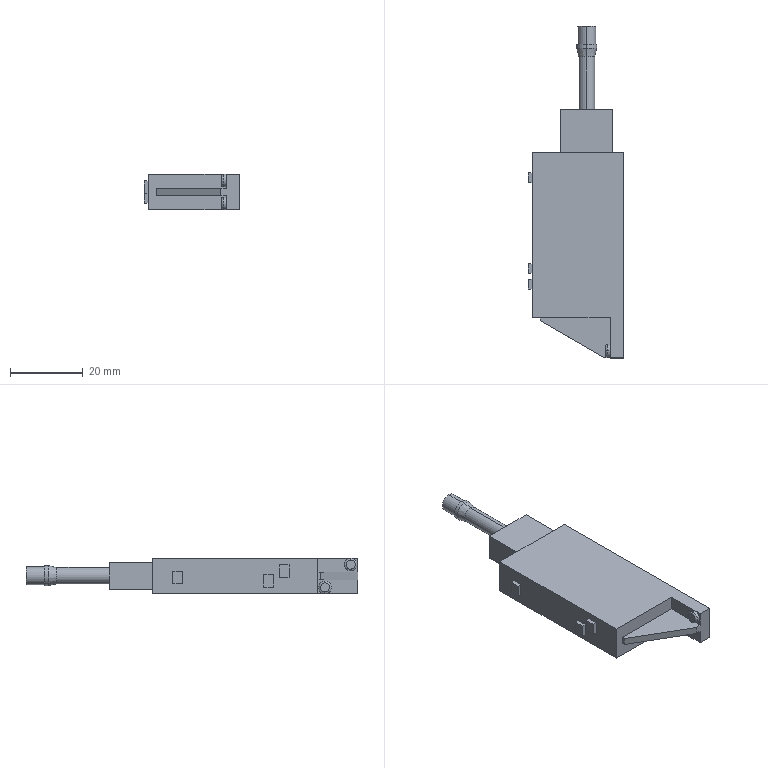Part | STEP file | 11-_ZK2-KAL_P-V2.0011 | 1 solid | 53 faces | box 26.3 x 91.5 x 9.8 mm | volume 13606 mm3 | plane 37 | cylinder 10 | spline 4 | cone 2 | commonest cylinder face diameters 3.5 x4 4.5 x2 4.92 x2 5.5 x2
STEP:
#1=CARTESIAN_POINT('',(-4.5,2.,4.9));
#2=VERTEX_POINT('',#1);
#3=CARTESIAN_POINT('',(-4.5,2.,1.4));
#4=VERTEX_POINT('',#3);
#5=CARTESIAN_POINT('',(-4.5,2.,3.15));
#6=DIRECTION('',(1.,0.,0.));
#7=DIRECTION('',(0.,0.,1.));
#8=AXIS2_PLACEMENT_3D('',#5,#6,#7);
#9=CIRCLE('',#8,1.75);
#10=EDGE_CURVE('',#2,#4,#9,.T.);
#11=ORIENTED_EDGE('',*,*,#10,.F.);
#12=CARTESIAN_POINT('',(-5.,2.,4.4));
#13=VERTEX_POINT('',#12);
#14=CARTESIAN_POINT('',(-4.5,2.,4.4));
#15=DIRECTION('',(0.,-1.,0.));
#16=DIRECTION('',(0.,0.,1.));
#17=AXIS2_PLACEMENT_3D('',#14,#15,#16);
#18=CIRCLE('',#17,0.5);
#19=EDGE_CURVE('',#2,#13,#18,.T.);
#20=ORIENTED_EDGE('',*,*,#19,.T.);
#21=CARTESIAN_POINT('',(-5.,2.,1.9));
#22=VERTEX_POINT('',#21);
#23=CARTESIAN_POINT('',(-5.,2.,4.4));
#24=CARTESIAN_POINT('',(-5.,-0.5,4.4));
#25=CARTESIAN_POINT('',(-5.,-0.5,1.9));
#26=CARTESIAN_POINT('',(-5.,2.,1.9));
#27=(BOUNDED_CURVE()B_SPLINE_CURVE(3,(#23,#24,#25,#26),.UNSPECIFIED.,.F.,.F.)B_SPLINE_CURVE_WITH_KNOTS((4,4),(0.5,1.),.UNSPECIFIED.)CURVE()GEOMETRIC_REPRESENTATION_ITEM()RATIONAL_B_SPLINE_CURVE((1.,0.3333,0.3333,1.))REPRESENTATION_ITEM(''));
#28=EDGE_CURVE('',#13,#22,#27,.T.);
#29=ORIENTED_EDGE('',*,*,#28,.T.);
#30=CARTESIAN_POINT('',(-4.5,2.,1.9));
#31=DIRECTION('',(0.,1.,0.));
#32=DIRECTION('',(0.,0.,-1.));
#33=AXIS2_PLACEMENT_3D('',#30,#31,#32);
#34=CIRCLE('',#33,0.5);
#35=EDGE_CURVE('',#4,#22,#34,.T.);
#36=ORIENTED_EDGE('',*,*,#35,.F.);
#37=EDGE_LOOP('',(#11,#20,#29,#36));
#38=FACE_OUTER_BOUND('',#37,.T.);
#39=CARTESIAN_POINT('',(-4.5,2.,4.9));
#40=CARTESIAN_POINT('',(-4.5,-1.5,4.9));
#41=CARTESIAN_POINT('',(-4.5,-1.5,1.4));
#42=CARTESIAN_POINT('',(-4.5,2.,1.4));
#43=CARTESIAN_POINT('',(-4.793,2.,4.9));
#44=CARTESIAN_POINT('',(-4.793,-1.5,4.9));
#45=CARTESIAN_POINT('',(-4.793,-1.5,1.4));
#46=CARTESIAN_POINT('',(-4.793,2.,1.4));
#47=CARTESIAN_POINT('',(-5.,2.,4.693));
#48=CARTESIAN_POINT('',(-5.,-1.086,4.693));
#49=CARTESIAN_POINT('',(-5.,-1.086,1.607));
#50=CARTESIAN_POINT('',(-5.,2.,1.607));
#51=CARTESIAN_POINT('',(-5.,2.,4.4));
#52=CARTESIAN_POINT('',(-5.,-0.5,4.4));
#53=CARTESIAN_POINT('',(-5.,-0.5,1.9));
#54=CARTESIAN_POINT('',(-5.,2.,1.9));
#55=(BOUNDED_SURFACE()B_SPLINE_SURFACE(3,3,((#39,#40,#41,#42),(#43,#44,#45,#46),(#47,#48,#49,#50),(#51,#52,#53,#54)),.UNSPECIFIED.,.F.,.F.,.F.)B_SPLINE_SURFACE_WITH_KNOTS((4,4),(4,4),(0.,1.),(0.,1.),.UNSPECIFIED.)GEOMETRIC_REPRESENTATION_ITEM()RATIONAL_B_SPLINE_SURFACE(((1.,0.3333,0.3333,1.),(0.8047,0.2682,0.2682,0.8047),(0.8047,0.2682,0.2682,0.8047),(1.,0.3333,0.3333,1.)))REPRESENTATION_ITEM('')SURFACE());
#56=ADVANCED_FACE('',(#38),#55,.T.);
#57=CARTESIAN_POINT('',(-4.5,9.1,-1.4));
#58=VERTEX_POINT('',#57);
#59=CARTESIAN_POINT('',(-4.5,9.1,-4.9));
#60=VERTEX_POINT('',#59);
#61=CARTESIAN_POINT('',(-4.5,9.1,-3.15));
#62=DIRECTION('',(1.,0.,0.));
#63=DIRECTION('',(0.,0.,1.));
#64=AXIS2_PLACEMENT_3D('',#61,#62,#63);
#65=CIRCLE('',#64,1.75);
#66=EDGE_CURVE('',#58,#60,#65,.T.);
#67=ORIENTED_EDGE('',*,*,#66,.F.);
#68=CARTESIAN_POINT('',(-5.,9.1,-1.9));
#69=VERTEX_POINT('',#68);
#70=CARTESIAN_POINT('',(-4.5,9.1,-1.9));
#71=DIRECTION('',(0.,-1.,0.));
#72=DIRECTION('',(0.,0.,1.));
#73=AXIS2_PLACEMENT_3D('',#70,#71,#72);
#74=CIRCLE('',#73,0.5);
#75=EDGE_CURVE('',#58,#69,#74,.T.);
#76=ORIENTED_EDGE('',*,*,#75,.T.);
#77=CARTESIAN_POINT('',(-5.,9.1,-4.4));
#78=VERTEX_POINT('',#77);
#79=CARTESIAN_POINT('',(-5.,9.1,-1.9));
#80=CARTESIAN_POINT('',(-5.,6.6,-1.9));
#81=CARTESIAN_POINT('',(-5.,6.6,-4.4));
#82=CARTESIAN_POINT('',(-5.,9.1,-4.4));
#83=(BOUNDED_CURVE()B_SPLINE_CURVE(3,(#79,#80,#81,#82),.UNSPECIFIED.,.F.,.F.)B_SPLINE_CURVE_WITH_KNOTS((4,4),(0.5,1.),.UNSPECIFIED.)CURVE()GEOMETRIC_REPRESENTATION_ITEM()RATIONAL_B_SPLINE_CURVE((1.,0.3333,0.3333,1.))REPRESENTATION_ITEM(''));
#84=EDGE_CURVE('',#69,#78,#83,.T.);
#85=ORIENTED_EDGE('',*,*,#84,.T.);
#86=CARTESIAN_POINT('',(-4.5,9.1,-4.4));
#87=DIRECTION('',(0.,1.,0.));
#88=DIRECTION('',(0.,0.,-1.));
#89=AXIS2_PLACEMENT_3D('',#86,#87,#88);
#90=CIRCLE('',#89,0.5);
#91=EDGE_CURVE('',#60,#78,#90,.T.);
#92=ORIENTED_EDGE('',*,*,#91,.F.);
#93=EDGE_LOOP('',(#67,#76,#85,#92));
#94=FACE_OUTER_BOUND('',#93,.T.);
#95=CARTESIAN_POINT('',(-4.5,9.1,-1.4));
#96=CARTESIAN_POINT('',(-4.5,5.6,-1.4));
#97=CARTESIAN_POINT('',(-4.5,5.6,-4.9));
#98=CARTESIAN_POINT('',(-4.5,9.1,-4.9));
#99=CARTESIAN_POINT('',(-4.793,9.1,-1.4));
#100=CARTESIAN_POINT('',(-4.793,5.6,-1.4));
#101=CARTESIAN_POINT('',(-4.793,5.6,-4.9));
#102=CARTESIAN_POINT('',(-4.793,9.1,-4.9));
#103=CARTESIAN_POINT('',(-5.,9.1,-1.607));
#104=CARTESIAN_POINT('',(-5.,6.014,-1.607));
#105=CARTESIAN_POINT('',(-5.,6.014,-4.693));
#106=CARTESIAN_POINT('',(-5.,9.1,-4.693));
#107=CARTESIAN_POINT('',(-5.,9.1,-1.9));
#108=CARTESIAN_POINT('',(-5.,6.6,-1.9));
#109=CARTESIAN_POINT('',(-5.,6.6,-4.4));
#110=CARTESIAN_POINT('',(-5.,9.1,-4.4));
#111=(BOUNDED_SURFACE()B_SPLINE_SURFACE(3,3,((#95,#96,#97,#98),(#99,#100,#101,#102),(#103,#104,#105,#106),(#107,#108,#109,#110)),.UNSPECIFIED.,.F.,.F.,.F.)B_SPLINE_SURFACE_WITH_KNOTS((4,4),(4,4),(0.,1.),(0.,1.),.UNSPECIFIED.)GEOMETRIC_REPRESENTATION_ITEM()RATIONAL_B_SPLINE_SURFACE(((1.,0.3333,0.3333,1.),(0.8047,0.2682,0.2682,0.8047),(0.8047,0.2682,0.2682,0.8047),(1.,0.3333,0.3333,1.)))REPRESENTATION_ITEM('')SURFACE());
#112=ADVANCED_FACE('',(#94),#111,.T.);
#113=CARTESIAN_POINT('',(-10.2,83.,-2.15));
#114=VERTEX_POINT('',#113);
#115=CARTESIAN_POINT('',(-10.2,83.,2.35));
#116=VERTEX_POINT('',#115);
#117=CARTESIAN_POINT('',(-10.2,83.,0.1));
#118=DIRECTION('',(0.,-1.,0.));
#119=DIRECTION('',(0.,0.,-1.));
#120=AXIS2_PLACEMENT_3D('',#117,#118,#119);
#121=CIRCLE('',#120,2.25);
#122=EDGE_CURVE('',#114,#116,#121,.T.);
#123=ORIENTED_EDGE('',*,*,#122,.T.);
#124=CARTESIAN_POINT('',(-10.2,68.5,2.35));
#125=VERTEX_POINT('',#124);
#126=CARTESIAN_POINT('',(-10.2,91.5,2.35));
#127=DIRECTION('',(0.,-1.,0.));
#128=VECTOR('',#127,1000.);
#129=LINE('',#126,#128);
#130=EDGE_CURVE('',#116,#125,#129,.T.);
#131=ORIENTED_EDGE('',*,*,#130,.T.);
#132=CARTESIAN_POINT('',(-10.2,68.5,-2.15));
#133=VERTEX_POINT('',#132);
#134=CARTESIAN_POINT('',(-10.2,68.5,0.1));
#135=DIRECTION('',(0.,1.,0.));
#136=DIRECTION('',(0.,0.,-1.));
#137=AXIS2_PLACEMENT_3D('',#134,#135,#136);
#138=CIRCLE('',#137,2.25);
#139=EDGE_CURVE('',#125,#133,#138,.T.);
#140=ORIENTED_EDGE('',*,*,#139,.T.);
#141=CARTESIAN_POINT('',(-10.2,91.5,-2.15));
#142=DIRECTION('',(0.,-1.,0.));
#143=VECTOR('',#142,1000.);
#144=LINE('',#141,#143);
#145=EDGE_CURVE('',#114,#133,#144,.T.);
#146=ORIENTED_EDGE('',*,*,#145,.F.);
#147=EDGE_LOOP('',(#123,#131,#140,#146));
#148=FACE_OUTER_BOUND('',#147,.T.);
#149=CARTESIAN_POINT('',(-10.2,91.5,0.1));
#150=DIRECTION('',(0.,-1.,0.));
#151=DIRECTION('',(0.,0.,-1.));
#152=AXIS2_PLACEMENT_3D('',#149,#150,#151);
#153=CYLINDRICAL_SURFACE('',#152,2.25);
#154=ADVANCED_FACE('',(#148),#153,.T.);
#155=ORIENTED_EDGE('',*,*,#122,.F.);
#156=CARTESIAN_POINT('',(-10.2,85.3,-2.65));
#157=VERTEX_POINT('',#156);
#158=CARTESIAN_POINT('',(-10.2,85.3,-2.65));
#159=DIRECTION('',(0.,0.9772,-0.2124));
#160=VECTOR('',#159,1000.);
#161=LINE('',#158,#160);
#162=EDGE_CURVE('',#114,#157,#161,.T.);
#163=ORIENTED_EDGE('',*,*,#162,.T.);
#164=CARTESIAN_POINT('',(-10.2,85.3,2.85));
#165=VERTEX_POINT('',#164);
#166=CARTESIAN_POINT('',(-10.2,85.3,0.1));
#167=DIRECTION('',(0.,-1.,0.));
#168=DIRECTION('',(0.,0.,1.));
#169=AXIS2_PLACEMENT_3D('',#166,#167,#168);
#170=CIRCLE('',#169,2.75);
#171=EDGE_CURVE('',#157,#165,#170,.T.);
#172=ORIENTED_EDGE('',*,*,#171,.T.);
#173=CARTESIAN_POINT('',(-10.2,85.3,2.85));
#174=DIRECTION('',(0.,0.9772,0.2124));
#175=VECTOR('',#174,1000.);
#176=LINE('',#173,#175);
#177=EDGE_CURVE('',#116,#165,#176,.T.);
#178=ORIENTED_EDGE('',*,*,#177,.F.);
#179=EDGE_LOOP('',(#155,#163,#172,#178));
#180=FACE_OUTER_BOUND('',#179,.T.);
#181=CARTESIAN_POINT('',(-10.2,85.3,0.1));
#182=DIRECTION('',(0.,1.,0.));
#183=DIRECTION('',(0.,0.,1.));
#184=AXIS2_PLACEMENT_3D('',#181,#182,#183);
#185=CONICAL_SURFACE('',#184,2.75,0.2141);
#186=ADVANCED_FACE('',(#180),#185,.T.);
#187=CARTESIAN_POINT('',(-10.2,86.5,-2.65));
#188=VERTEX_POINT('',#187);
#189=CARTESIAN_POINT('',(-10.2,86.5,2.85));
#190=VERTEX_POINT('',#189);
#191=CARTESIAN_POINT('',(-10.2,86.5,0.1));
#192=DIRECTION('',(0.,-1.,0.));
#193=DIRECTION('',(0.,0.,-1.));
#194=AXIS2_PLACEMENT_3D('',#191,#192,#193);
#195=CIRCLE('',#194,2.75);
#196=EDGE_CURVE('',#188,#190,#195,.T.);
#197=ORIENTED_EDGE('',*,*,#196,.T.);
#198=CARTESIAN_POINT('',(-10.2,91.5,2.85));
#199=DIRECTION('',(0.,-1.,0.));
#200=VECTOR('',#199,1000.);
#201=LINE('',#198,#200);
#202=EDGE_CURVE('',#190,#165,#201,.T.);
#203=ORIENTED_EDGE('',*,*,#202,.T.);
#204=ORIENTED_EDGE('',*,*,#171,.F.);
#205=CARTESIAN_POINT('',(-10.2,91.5,-2.65));
#206=DIRECTION('',(0.,-1.,0.));
#207=VECTOR('',#206,1000.);
#208=LINE('',#205,#207);
#209=EDGE_CURVE('',#188,#157,#208,.T.);
#210=ORIENTED_EDGE('',*,*,#209,.F.);
#211=EDGE_LOOP('',(#197,#203,#204,#210));
#212=FACE_OUTER_BOUND('',#211,.T.);
#213=CARTESIAN_POINT('',(-10.2,91.5,0.1));
#214=DIRECTION('',(0.,-1.,0.));
#215=DIRECTION('',(0.,0.,-1.));
#216=AXIS2_PLACEMENT_3D('',#213,#214,#215);
#217=CYLINDRICAL_SURFACE('',#216,2.75);
#218=ADVANCED_FACE('',(#212),#217,.T.);
#219=CARTESIAN_POINT('',(-10.2,91.5,-2.36));
#220=VERTEX_POINT('',#219);
#221=CARTESIAN_POINT('',(-10.2,91.5,2.56));
#222=VERTEX_POINT('',#221);
#223=CARTESIAN_POINT('',(-10.2,91.5,0.1));
#224=DIRECTION('',(0.,-1.,0.));
#225=DIRECTION('',(0.,0.,-1.));
#226=AXIS2_PLACEMENT_3D('',#223,#224,#225);
#227=CIRCLE('',#226,2.46);
#228=EDGE_CURVE('',#220,#222,#227,.T.);
#229=ORIENTED_EDGE('',*,*,#228,.T.);
#230=CARTESIAN_POINT('',(-10.2,86.5,2.56));
#231=VERTEX_POINT('',#230);
#232=CARTESIAN_POINT('',(-10.2,91.5,2.56));
#233=DIRECTION('',(0.,-1.,0.));
#234=VECTOR('',#233,1000.);
#235=LINE('',#232,#234);
#236=EDGE_CURVE('',#222,#231,#235,.T.);
#237=ORIENTED_EDGE('',*,*,#236,.T.);
#238=CARTESIAN_POINT('',(-10.2,86.5,-2.36));
#239=VERTEX_POINT('',#238);
#240=CARTESIAN_POINT('',(-10.2,86.5,0.1));
#241=DIRECTION('',(0.,1.,0.));
#242=DIRECTION('',(0.,0.,-1.));
#243=AXIS2_PLACEMENT_3D('',#240,#241,#242);
#244=CIRCLE('',#243,2.46);
#245=EDGE_CURVE('',#231,#239,#244,.T.);
#246=ORIENTED_EDGE('',*,*,#245,.T.);
#247=CARTESIAN_POINT('',(-10.2,91.5,-2.36));
#248=DIRECTION('',(0.,-1.,0.));
#249=VECTOR('',#248,1000.);
#250=LINE('',#247,#249);
#251=EDGE_CURVE('',#220,#239,#250,.T.);
#252=ORIENTED_EDGE('',*,*,#251,.F.);
#253=EDGE_LOOP('',(#229,#237,#246,#252));
#254=FACE_OUTER_BOUND('',#253,.T.);
#255=CARTESIAN_POINT('',(-10.2,91.5,0.1));
#256=DIRECTION('',(0.,-1.,0.));
#257=DIRECTION('',(0.,0.,-1.));
#258=AXIS2_PLACEMENT_3D('',#255,#256,#257);
#259=CYLINDRICAL_SURFACE('',#258,2.46);
#260=ADVANCED_FACE('',(#254),#259,.T.);
#261=CARTESIAN_POINT('',(-3.7,2.,4.9));
#262=VERTEX_POINT('',#261);
#263=CARTESIAN_POINT('',(-3.7,2.,1.4));
#264=VERTEX_POINT('',#263);
#265=CARTESIAN_POINT('',(-3.7,2.,3.15));
#266=DIRECTION('',(-1.,0.,0.));
#267=DIRECTION('',(0.,0.,1.));
#268=AXIS2_PLACEMENT_3D('',#265,#266,#267);
#269=CIRCLE('',#268,1.75);
#270=EDGE_CURVE('',#262,#264,#269,.T.);
#271=ORIENTED_EDGE('',*,*,#270,.T.);
#272=CARTESIAN_POINT('',(-3.7,2.,1.4));
#273=DIRECTION('',(-1.,0.,0.));
#274=VECTOR('',#273,1000.);
#275=LINE('',#272,#274);
#276=EDGE_CURVE('',#264,#4,#275,.T.);
#277=ORIENTED_EDGE('',*,*,#276,.T.);
#278=CARTESIAN_POINT('',(-4.5,2.,3.15));
#279=DIRECTION('',(1.,0.,0.));
#280=DIRECTION('',(0.,0.,1.));
#281=AXIS2_PLACEMENT_3D('',#278,#279,#280);
#282=CIRCLE('',#281,1.75);
#283=EDGE_CURVE('',#4,#2,#282,.T.);
#284=ORIENTED_EDGE('',*,*,#283,.T.);
#285=CARTESIAN_POINT('',(-3.7,2.,4.9));
#286=DIRECTION('',(-1.,0.,0.));
#287=VECTOR('',#286,1000.);
#288=LINE('',#285,#287);
#289=EDGE_CURVE('',#262,#2,#288,.T.);
#290=ORIENTED_EDGE('',*,*,#289,.F.);
#291=EDGE_LOOP('',(#271,#277,#284,#290));
#292=FACE_OUTER_BOUND('',#291,.T.);
#293=CARTESIAN_POINT('',(-3.7,2.,3.15));
#294=DIRECTION('',(-1.,0.,0.));
#295=DIRECTION('',(0.,0.,1.));
#296=AXIS2_PLACEMENT_3D('',#293,#294,#295);
#297=CYLINDRICAL_SURFACE('',#296,1.75);
#298=ADVANCED_FACE('',(#292),#297,.T.);
#299=CARTESIAN_POINT('',(-3.7,9.1,-1.4));
#300=VERTEX_POINT('',#299);
#301=CARTESIAN_POINT('',(-3.7,9.1,-4.9));
#302=VERTEX_POINT('',#301);
#303=CARTESIAN_POINT('',(-3.7,9.1,-3.15));
#304=DIRECTION('',(-1.,0.,0.));
#305=DIRECTION('',(0.,0.,1.));
#306=AXIS2_PLACEMENT_3D('',#303,#304,#305);
#307=CIRCLE('',#306,1.75);
#308=EDGE_CURVE('',#300,#302,#307,.T.);
#309=ORIENTED_EDGE('',*,*,#308,.T.);
#310=CARTESIAN_POINT('',(-3.7,9.1,-4.9));
#311=DIRECTION('',(-1.,0.,0.));
#312=VECTOR('',#311,1000.);
#313=LINE('',#310,#312);
#314=EDGE_CURVE('',#302,#60,#313,.T.);
#315=ORIENTED_EDGE('',*,*,#314,.T.);
#316=CARTESIAN_POINT('',(-4.5,9.1,-3.15));
#317=DIRECTION('',(1.,0.,0.));
#318=DIRECTION('',(0.,0.,1.));
#319=AXIS2_PLACEMENT_3D('',#316,#317,#318);
#320=CIRCLE('',#319,1.75);
#321=EDGE_CURVE('',#60,#58,#320,.T.);
#322=ORIENTED_EDGE('',*,*,#321,.T.);
#323=CARTESIAN_POINT('',(-3.7,9.1,-1.4));
#324=DIRECTION('',(-1.,0.,0.));
#325=VECTOR('',#324,1000.);
#326=LINE('',#323,#325);
#327=EDGE_CURVE('',#300,#58,#326,.T.);
#328=ORIENTED_EDGE('',*,*,#327,.F.);
#329=EDGE_LOOP('',(#309,#315,#322,#328));
#330=FACE_OUTER_BOUND('',#329,.T.);
#331=CARTESIAN_POINT('',(-3.7,9.1,-3.15));
#332=DIRECTION('',(-1.,0.,0.));
#333=DIRECTION('',(0.,0.,1.));
#334=AXIS2_PLACEMENT_3D('',#331,#332,#333);
#335=CYLINDRICAL_SURFACE('',#334,1.75);
#336=ADVANCED_FACE('',(#330),#335,.T.);
#337=CARTESIAN_POINT('',(-3.7,11.1,4.9));
#338=VERTEX_POINT('',#337);
#339=CARTESIAN_POINT('',(-3.7,2.,4.9));
#340=CARTESIAN_POINT('',(-3.7,11.1,4.9));
#341=B_SPLINE_CURVE_WITH_KNOTS('',1,(#339,#340),.UNSPECIFIED.,.F.,.F.,(2,2),(0.1802,1.),.UNSPECIFIED.);
#342=EDGE_CURVE('',#262,#338,#341,.T.);
#343=ORIENTED_EDGE('',*,*,#342,.T.);
#344=CARTESIAN_POINT('',(-3.7,11.1,1.));
#345=VERTEX_POINT('',#344);
#346=CARTESIAN_POINT('',(-3.7,11.1,4.9));
#347=CARTESIAN_POINT('',(-3.7,11.1,1.));
#348=B_SPLINE_CURVE_WITH_KNOTS('',1,(#346,#347),.UNSPECIFIED.,.F.,.F.,(2,2),(0.,1.),.UNSPECIFIED.);
#349=EDGE_CURVE('',#338,#345,#348,.T.);
#350=ORIENTED_EDGE('',*,*,#349,.T.);
#351=CARTESIAN_POINT('',(-3.7,0.,1.));
#352=VERTEX_POINT('',#351);
#353=CARTESIAN_POINT('',(-3.7,0.,1.));
#354=CARTESIAN_POINT('',(-3.7,11.1,1.));
#355=B_SPLINE_CURVE_WITH_KNOTS('',1,(#353,#354),.UNSPECIFIED.,.F.,.F.,(2,2),(0.,1.),.UNSPECIFIED.);
#356=EDGE_CURVE('',#352,#345,#355,.T.);
#357=ORIENTED_EDGE('',*,*,#356,.F.);
#358=CARTESIAN_POINT('',(-3.7,0.,4.9));
#359=VERTEX_POINT('',#358);
#360=CARTESIAN_POINT('',(-3.7,0.,4.9));
#361=CARTESIAN_POINT('',(-3.7,0.,1.));
#362=B_SPLINE_CURVE_WITH_KNOTS('',1,(#360,#361),.UNSPECIFIED.,.F.,.F.,(2,2),(0.,1.),.UNSPECIFIED.);
#363=EDGE_CURVE('',#359,#352,#362,.T.);
#364=ORIENTED_EDGE('',*,*,#363,.F.);
#365=CARTESIAN_POINT('',(-3.7,0.,4.9));
#366=CARTESIAN_POINT('',(-3.7,2.,4.9));
#367=B_SPLINE_CURVE_WITH_KNOTS('',1,(#365,#366),.UNSPECIFIED.,.F.,.F.,(2,2),(0.,0.1802),.UNSPECIFIED.);
#368=EDGE_CURVE('',#359,#262,#367,.T.);
#369=ORIENTED_EDGE('',*,*,#368,.T.);
#370=CARTESIAN_POINT('',(-3.7,2.,3.15));
#371=DIRECTION('',(-1.,0.,0.));
#372=DIRECTION('',(0.,0.,1.));
#373=AXIS2_PLACEMENT_3D('',#370,#371,#372);
#374=CIRCLE('',#373,1.75);
#375=EDGE_CURVE('',#264,#262,#374,.T.);
#376=ORIENTED_EDGE('',*,*,#375,.F.);
#377=ORIENTED_EDGE('',*,*,#270,.F.);
#378=EDGE_LOOP('',(#343,#350,#357,#364,#369,#376,#377));
#379=FACE_OUTER_BOUND('',#378,.T.);
#380=CARTESIAN_POINT('',(-3.7,11.1,4.9));
#381=DIRECTION('',(1.,0.,0.));
#382=DIRECTION('',(0.,0.,-1.));
#383=AXIS2_PLACEMENT_3D('',#380,#381,#382);
#384=PLANE('',#383);
#385=ADVANCED_FACE('',(#379),#384,.F.);
#386=CARTESIAN_POINT('',(-26.3,21.7,-0.35));
#387=VERTEX_POINT('',#386);
#388=CARTESIAN_POINT('',(-26.3,21.7,3.05));
#389=VERTEX_POINT('',#388);
#390=CARTESIAN_POINT('',(-26.3,21.7,-0.35));
#391=DIRECTION('',(0.,0.,1.));
#392=VECTOR('',#391,1000.);
#393=LINE('',#390,#392);
#394=EDGE_CURVE('',#387,#389,#393,.T.);
#395=ORIENTED_EDGE('',*,*,#394,.F.);
#396=CARTESIAN_POINT('',(-26.3,19.,-0.35));
#397=VERTEX_POINT('',#396);
#398=CARTESIAN_POINT('',(-26.3,19.,-0.35));
#399=DIRECTION('',(0.,1.,0.));
#400=VECTOR('',#399,1000.);
#401=LINE('',#398,#400);
#402=EDGE_CURVE('',#397,#387,#401,.T.);
#403=ORIENTED_EDGE('',*,*,#402,.F.);
#404=CARTESIAN_POINT('',(-26.3,19.,3.05));
#405=VERTEX_POINT('',#404);
#406=CARTESIAN_POINT('',(-26.3,19.,3.05));
#407=DIRECTION('',(0.,0.,-1.));
#408=VECTOR('',#407,1000.);
#409=LINE('',#406,#408);
#410=EDGE_CURVE('',#405,#397,#409,.T.);
#411=ORIENTED_EDGE('',*,*,#410,.F.);
#412=CARTESIAN_POINT('',(-26.3,21.7,3.05));
#413=DIRECTION('',(0.,-1.,0.));
#414=VECTOR('',#413,1000.);
#415=LINE('',#412,#414);
#416=EDGE_CURVE('',#389,#405,#415,.T.);
#417=ORIENTED_EDGE('',*,*,#416,.F.);
#418=EDGE_LOOP('',(#395,#403,#411,#417));
#419=FACE_OUTER_BOUND('',#418,.T.);
#420=CARTESIAN_POINT('',(-26.3,0.,0.));
#421=DIRECTION('',(1.,0.,0.));
#422=DIRECTION('',(0.,0.,-1.));
#423=AXIS2_PLACEMENT_3D('',#420,#421,#422);
#424=PLANE('',#423);
#425=ADVANCED_FACE('',(#419),#424,.F.);
#426=CARTESIAN_POINT('',(-26.3,26.,-3.05));
#427=VERTEX_POINT('',#426);
#428=CARTESIAN_POINT('',(-26.3,26.,0.35));
#429=VERTEX_POINT('',#428);
#430=CARTESIAN_POINT('',(-26.3,26.,-3.05));
#431=DIRECTION('',(0.,0.,1.));
#432=VECTOR('',#431,1000.);
#433=LINE('',#430,#432);
#434=EDGE_CURVE('',#427,#429,#433,.T.);
#435=ORIENTED_EDGE('',*,*,#434,.F.);
#436=CARTESIAN_POINT('',(-26.3,23.3,-3.05));
#437=VERTEX_POINT('',#436);
#438=CARTESIAN_POINT('',(-26.3,23.3,-3.05));
#439=DIRECTION('',(0.,1.,0.));
#440=VECTOR('',#439,1000.);
#441=LINE('',#438,#440);
#442=EDGE_CURVE('',#437,#427,#441,.T.);
#443=ORIENTED_EDGE('',*,*,#442,.F.);
#444=CARTESIAN_POINT('',(-26.3,23.3,0.35));
#445=VERTEX_POINT('',#444);
#446=CARTESIAN_POINT('',(-26.3,23.3,0.35));
#447=DIRECTION('',(0.,0.,-1.));
#448=VECTOR('',#447,1000.);
#449=LINE('',#446,#448);
#450=EDGE_CURVE('',#445,#437,#449,.T.);
#451=ORIENTED_EDGE('',*,*,#450,.F.);
#452=CARTESIAN_POINT('',(-26.3,26.,0.35));
#453=DIRECTION('',(0.,-1.,0.));
#454=VECTOR('',#453,1000.);
#455=LINE('',#452,#454);
#456=EDGE_CURVE('',#429,#445,#455,.T.);
#457=ORIENTED_EDGE('',*,*,#456,.F.);
#458=EDGE_LOOP('',(#435,#443,#451,#457));
#459=FACE_OUTER_BOUND('',#458,.T.);
#460=CARTESIAN_POINT('',(-26.3,4.3,-2.7));
#461=DIRECTION('',(1.,0.,0.));
#462=DIRECTION('',(0.,0.,-1.));
#463=AXIS2_PLACEMENT_3D('',#460,#461,#462);
#464=PLANE('',#463);
#465=ADVANCED_FACE('',(#459),#464,.F.);
#466=CARTESIAN_POINT('',(-26.3,51.05,-2.05));
#467=VERTEX_POINT('',#466);
#468=CARTESIAN_POINT('',(-26.3,51.05,1.35));
#469=VERTEX_POINT('',#468);
#470=CARTESIAN_POINT('',(-26.3,51.05,-2.05));
#471=DIRECTION('',(0.,0.,1.));
#472=VECTOR('',#471,1000.);
#473=LINE('',#470,#472);
#474=EDGE_CURVE('',#467,#469,#473,.T.);
#475=ORIENTED_EDGE('',*,*,#474,.F.);
#476=CARTESIAN_POINT('',(-26.3,48.35,-2.05));
#477=VERTEX_POINT('',#476);
#478=CARTESIAN_POINT('',(-26.3,48.35,-2.05));
#479=DIRECTION('',(0.,1.,0.));
#480=VECTOR('',#479,1000.);
#481=LINE('',#478,#480);
#482=EDGE_CURVE('',#477,#467,#481,.T.);
#483=ORIENTED_EDGE('',*,*,#482,.F.);
#484=CARTESIAN_POINT('',(-26.3,48.35,1.35));
#485=VERTEX_POINT('',#484);
#486=CARTESIAN_POINT('',(-26.3,48.35,1.35));
#487=DIRECTION('',(0.,0.,-1.));
#488=VECTOR('',#487,1000.);
#489=LINE('',#486,#488);
#490=EDGE_CURVE('',#485,#477,#489,.T.);
#491=ORIENTED_EDGE('',*,*,#490,.F.);
#492=CARTESIAN_POINT('',(-26.3,51.05,1.35));
#493=DIRECTION('',(0.,-1.,0.));
#494=VECTOR('',#493,1000.);
#495=LINE('',#492,#494);
#496=EDGE_CURVE('',#469,#485,#495,.T.);
#497=ORIENTED_EDGE('',*,*,#496,.F.);
#498=EDGE_LOOP('',(#475,#483,#491,#497));
#499=FACE_OUTER_BOUND('',#498,.T.);
#500=CARTESIAN_POINT('',(-26.3,29.35,-1.7));
#501=DIRECTION('',(1.,0.,0.));
#502=DIRECTION('',(0.,0.,-1.));
#503=AXIS2_PLACEMENT_3D('',#500,#501,#502);
#504=PLANE('',#503);
#505=ADVANCED_FACE('',(#499),#504,.F.);
#506=CARTESIAN_POINT('',(-10.2,68.5,0.1));
#507=DIRECTION('',(0.,1.,0.));
#508=DIRECTION('',(0.,0.,-1.));
#509=AXIS2_PLACEMENT_3D('',#506,#507,#508);
#510=CIRCLE('',#509,2.25);
#511=EDGE_CURVE('',#133,#125,#510,.T.);
#512=ORIENTED_EDGE('',*,*,#511,.F.);
#513=ORIENTED_EDGE('',*,*,#139,.F.);
#514=EDGE_LOOP('',(#512,#513));
#515=FACE_BOUND('',#514,.T.);
#516=CARTESIAN_POINT('',(-17.4,68.5,3.7));
#517=VERTEX_POINT('',#516);
#518=CARTESIAN_POINT('',(-3.,68.5,3.7));
#519=VERTEX_POINT('',#518);
#520=CARTESIAN_POINT('',(-3.,68.5,3.7));
#521=DIRECTION('',(1.,0.,0.));
#522=VECTOR('',#521,1000.);
#523=LINE('',#520,#522);
#524=EDGE_CURVE('',#517,#519,#523,.T.);
#525=ORIENTED_EDGE('',*,*,#524,.T.);
#526=CARTESIAN_POINT('',(-3.,68.5,-3.7));
#527=VERTEX_POINT('',#526);
#528=CARTESIAN_POINT('',(-3.,68.5,0.));
#529=DIRECTION('',(0.,0.,1.));
#530=VECTOR('',#529,1000.);
#531=LINE('',#528,#530);
#532=EDGE_CURVE('',#527,#519,#531,.T.);
#533=ORIENTED_EDGE('',*,*,#532,.F.);
#534=CARTESIAN_POINT('',(-17.4,68.5,-3.7));
#535=VERTEX_POINT('',#534);
#536=CARTESIAN_POINT('',(-3.,68.5,-3.7));
#537=DIRECTION('',(-1.,0.,0.));
#538=VECTOR('',#537,1000.);
#539=LINE('',#536,#538);
#540=EDGE_CURVE('',#527,#535,#539,.T.);
#541=ORIENTED_EDGE('',*,*,#540,.T.);
#542=CARTESIAN_POINT('',(-17.4,68.5,0.));
#543=DIRECTION('',(0.,0.,1.));
#544=VECTOR('',#543,1000.);
#545=LINE('',#542,#544);
#546=EDGE_CURVE('',#535,#517,#545,.T.);
#547=ORIENTED_EDGE('',*,*,#546,.T.);
#548=EDGE_LOOP('',(#525,#533,#541,#547));
#549=FACE_OUTER_BOUND('',#548,.T.);
#550=CARTESIAN_POINT('',(-3.,68.5,-3.7));
#551=DIRECTION('',(0.,-1.,0.));
#552=DIRECTION('',(0.,0.,-1.));
#553=AXIS2_PLACEMENT_3D('',#550,#551,#552);
#554=PLANE('',#553);
#555=ADVANCED_FACE('',(#515,#549),#554,.F.);
#556=ORIENTED_EDGE('',*,*,#130,.F.);
#557=CARTESIAN_POINT('',(-10.2,83.,0.1));
#558=DIRECTION('',(0.,-1.,0.));
#559=DIRECTION('',(0.,0.,-1.));
#560=AXIS2_PLACEMENT_3D('',#557,#558,#559);
#561=CIRCLE('',#560,2.25);
#562=EDGE_CURVE('',#116,#114,#561,.T.);
#563=ORIENTED_EDGE('',*,*,#562,.T.);
#564=ORIENTED_EDGE('',*,*,#145,.T.);
#565=ORIENTED_EDGE('',*,*,#511,.T.);
#566=EDGE_LOOP('',(#556,#563,#564,#565));
#567=FACE_OUTER_BOUND('',#566,.T.);
#568=CARTESIAN_POINT('',(-10.2,91.5,0.1));
#569=DIRECTION('',(0.,-1.,0.));
#570=DIRECTION('',(0.,0.,-1.));
#571=AXIS2_PLACEMENT_3D('',#568,#569,#570);
#572=CYLINDRICAL_SURFACE('',#571,2.25);
#573=ADVANCED_FACE('',(#567),#572,.T.);
#574=ORIENTED_EDGE('',*,*,#162,.F.);
#575=ORIENTED_EDGE('',*,*,#562,.F.);
#576=ORIENTED_EDGE('',*,*,#177,.T.);
#577=CARTESIAN_POINT('',(-10.2,85.3,0.1));
#578=DIRECTION('',(0.,-1.,0.));
#579=DIRECTION('',(0.,0.,1.));
#580=AXIS2_PLACEMENT_3D('',#577,#578,#579);
#581=CIRCLE('',#580,2.75);
#582=EDGE_CURVE('',#165,#157,#581,.T.);
#583=ORIENTED_EDGE('',*,*,#582,.T.);
#584=EDGE_LOOP('',(#574,#575,#576,#583));
#585=FACE_OUTER_BOUND('',#584,.T.);
#586=CARTESIAN_POINT('',(-10.2,85.3,0.1));
#587=DIRECTION('',(0.,1.,0.));
#588=DIRECTION('',(0.,0.,1.));
#589=AXIS2_PLACEMENT_3D('',#586,#587,#588);
#590=CONICAL_SURFACE('',#589,2.75,0.2141);
#591=ADVANCED_FACE('',(#585),#590,.T.);
#592=ORIENTED_EDGE('',*,*,#202,.F.);
#593=CARTESIAN_POINT('',(-10.2,86.5,0.1));
#594=DIRECTION('',(0.,-1.,0.));
#595=DIRECTION('',(0.,0.,-1.));
#596=AXIS2_PLACEMENT_3D('',#593,#594,#595);
#597=CIRCLE('',#596,2.75);
#598=EDGE_CURVE('',#190,#188,#597,.T.);
#599=ORIENTED_EDGE('',*,*,#598,.T.);
#600=ORIENTED_EDGE('',*,*,#209,.T.);
#601=ORIENTED_EDGE('',*,*,#582,.F.);
#602=EDGE_LOOP('',(#592,#599,#600,#601));
#603=FACE_OUTER_BOUND('',#602,.T.);
#604=CARTESIAN_POINT('',(-10.2,91.5,0.1));
#605=DIRECTION('',(0.,-1.,0.));
#606=DIRECTION('',(0.,0.,-1.));
#607=AXIS2_PLACEMENT_3D('',#604,#605,#606);
#608=CYLINDRICAL_SURFACE('',#607,2.75);
#609=ADVANCED_FACE('',(#603),#608,.T.);
#610=ORIENTED_EDGE('',*,*,#196,.F.);
#611=ORIENTED_EDGE('',*,*,#598,.F.);
#612=EDGE_LOOP('',(#610,#611));
#613=FACE_OUTER_BOUND('',#612,.T.);
#614=CARTESIAN_POINT('',(-10.2,86.5,0.1));
#615=DIRECTION('',(0.,1.,0.));
#616=DIRECTION('',(0.,0.,-1.));
#617=AXIS2_PLACEMENT_3D('',#614,#615,#616);
#618=CIRCLE('',#617,2.46);
#619=EDGE_CURVE('',#239,#231,#618,.T.);
#620=ORIENTED_EDGE('',*,*,#619,.F.);
#621=ORIENTED_EDGE('',*,*,#245,.F.);
#622=EDGE_LOOP('',(#620,#621));
#623=FACE_BOUND('',#622,.T.);
#624=CARTESIAN_POINT('',(-10.2,86.5,2.85));
#625=DIRECTION('',(0.,-1.,0.));
#626=DIRECTION('',(0.,0.,-1.));
#627=AXIS2_PLACEMENT_3D('',#624,#625,#626);
#628=PLANE('',#627);
#629=ADVANCED_FACE('',(#613,#623),#628,.F.);
#630=ORIENTED_EDGE('',*,*,#236,.F.);
#631=CARTESIAN_POINT('',(-10.2,91.5,0.1));
#632=DIRECTION('',(0.,-1.,0.));
#633=DIRECTION('',(0.,0.,-1.));
#634=AXIS2_PLACEMENT_3D('',#631,#632,#633);
#635=CIRCLE('',#634,2.46);
#636=EDGE_CURVE('',#222,#220,#635,.T.);
#637=ORIENTED_EDGE('',*,*,#636,.T.);
#638=ORIENTED_EDGE('',*,*,#251,.T.);
#639=ORIENTED_EDGE('',*,*,#619,.T.);
#640=EDGE_LOOP('',(#630,#637,#638,#639));
#641=FACE_OUTER_BOUND('',#640,.T.);
#642=CARTESIAN_POINT('',(-10.2,91.5,0.1));
#643=DIRECTION('',(0.,-1.,0.));
#644=DIRECTION('',(0.,0.,-1.));
#645=AXIS2_PLACEMENT_3D('',#642,#643,#644);
#646=CYLINDRICAL_SURFACE('',#645,2.46);
#647=ADVANCED_FACE('',(#641),#646,.T.);
#648=ORIENTED_EDGE('',*,*,#228,.F.);
#649=ORIENTED_EDGE('',*,*,#636,.F.);
#650=EDGE_LOOP('',(#648,#649));
#651=FACE_OUTER_BOUND('',#650,.T.);
#652=CARTESIAN_POINT('',(-10.2,91.5,2.56));
#653=DIRECTION('',(0.,-1.,0.));
#654=DIRECTION('',(0.,0.,-1.));
#655=AXIS2_PLACEMENT_3D('',#652,#653,#654);
#656=PLANE('',#655);
#657=ADVANCED_FACE('',(#651),#656,.F.);
#658=ORIENTED_EDGE('',*,*,#474,.T.);
#659=CARTESIAN_POINT('',(-25.2,51.05,1.35));
#660=VERTEX_POINT('',#659);
#661=CARTESIAN_POINT('',(-26.3,51.05,1.35));
#662=DIRECTION('',(1.,0.,0.));
#663=VECTOR('',#662,1000.);
#664=LINE('',#661,#663);
#665=EDGE_CURVE('',#469,#660,#664,.T.);
#666=ORIENTED_EDGE('',*,*,#665,.T.);
#667=CARTESIAN_POINT('',(-25.2,51.05,-2.05));
#668=VERTEX_POINT('',#667);
#669=CARTESIAN_POINT('',(-25.2,51.05,4.9));
#670=DIRECTION('',(0.,0.,-1.));
#671=VECTOR('',#670,1000.);
#672=LINE('',#669,#671);
#673=EDGE_CURVE('',#660,#668,#672,.T.);
#674=ORIENTED_EDGE('',*,*,#673,.T.);
#675=CARTESIAN_POINT('',(-26.3,51.05,-2.05));
#676=DIRECTION('',(-1.,0.,0.));
#677=VECTOR('',#676,1000.);
#678=LINE('',#675,#677);
#679=EDGE_CURVE('',#668,#467,#678,.T.);
#680=ORIENTED_EDGE('',*,*,#679,.T.);
#681=EDGE_LOOP('',(#658,#666,#674,#680));
#682=FACE_OUTER_BOUND('',#681,.T.);
#683=CARTESIAN_POINT('',(-26.3,51.05,-2.05));
#684=DIRECTION('',(0.,1.,0.));
#685=DIRECTION('',(0.,0.,1.));
#686=AXIS2_PLACEMENT_3D('',#683,#684,#685);
#687=PLANE('',#686);
#688=ADVANCED_FACE('',(#682),#687,.T.);
#689=ORIENTED_EDGE('',*,*,#482,.T.);
#690=ORIENTED_EDGE('',*,*,#679,.F.);
#691=CARTESIAN_POINT('',(-25.2,48.35,-2.05));
#692=VERTEX_POINT('',#691);
#693=CARTESIAN_POINT('',(-25.2,56.6,-2.05));
#694=DIRECTION('',(0.,-1.,0.));
#695=VECTOR('',#694,1000.);
#696=LINE('',#693,#695);
#697=EDGE_CURVE('',#668,#692,#696,.T.);
#698=ORIENTED_EDGE('',*,*,#697,.T.);
#699=CARTESIAN_POINT('',(-26.3,48.35,-2.05));
#700=DIRECTION('',(1.,0.,0.));
#701=VECTOR('',#700,1000.);
#702=LINE('',#699,#701);
#703=EDGE_CURVE('',#477,#692,#702,.T.);
#704=ORIENTED_EDGE('',*,*,#703,.F.);
#705=EDGE_LOOP('',(#689,#690,#698,#704));
#706=FACE_OUTER_BOUND('',#705,.T.);
#707=CARTESIAN_POINT('',(-26.3,48.35,-2.05));
#708=DIRECTION('',(0.,0.,-1.));
#709=DIRECTION('',(0.,1.,0.));
#710=AXIS2_PLACEMENT_3D('',#707,#708,#709);
#711=PLANE('',#710);
#712=ADVANCED_FACE('',(#706),#711,.T.);
#713=ORIENTED_EDGE('',*,*,#490,.T.);
#714=ORIENTED_EDGE('',*,*,#703,.T.);
#715=CARTESIAN_POINT('',(-25.2,48.35,1.35));
#716=VERTEX_POINT('',#715);
#717=CARTESIAN_POINT('',(-25.2,48.35,4.9));
#718=DIRECTION('',(0.,0.,1.));
#719=VECTOR('',#718,1000.);
#720=LINE('',#717,#719);
#721=EDGE_CURVE('',#692,#716,#720,.T.);
#722=ORIENTED_EDGE('',*,*,#721,.T.);
#723=CARTESIAN_POINT('',(-26.3,48.35,1.35));
#724=DIRECTION('',(1.,0.,0.));
#725=VECTOR('',#724,1000.);
#726=LINE('',#723,#725);
#727=EDGE_CURVE('',#485,#716,#726,.T.);
#728=ORIENTED_EDGE('',*,*,#727,.F.);
#729=EDGE_LOOP('',(#713,#714,#722,#728));
#730=FACE_OUTER_BOUND('',#729,.T.);
#731=CARTESIAN_POINT('',(-26.3,48.35,1.35));
#732=DIRECTION('',(0.,-1.,0.));
#733=DIRECTION('',(0.,0.,-1.));
#734=AXIS2_PLACEMENT_3D('',#731,#732,#733);
#735=PLANE('',#734);
#736=ADVANCED_FACE('',(#730),#735,.T.);
#737=ORIENTED_EDGE('',*,*,#496,.T.);
#738=ORIENTED_EDGE('',*,*,#727,.T.);
#739=CARTESIAN_POINT('',(-25.2,56.6,1.35));
#740=DIRECTION('',(0.,1.,0.));
#741=VECTOR('',#740,1000.);
#742=LINE('',#739,#741);
#743=EDGE_CURVE('',#716,#660,#742,.T.);
#744=ORIENTED_EDGE('',*,*,#743,.T.);
#745=ORIENTED_EDGE('',*,*,#665,.F.);
#746=EDGE_LOOP('',(#737,#738,#744,#745));
#747=FACE_OUTER_BOUND('',#746,.T.);
#748=CARTESIAN_POINT('',(-26.3,51.05,1.35));
#749=DIRECTION('',(0.,0.,1.));
#750=DIRECTION('',(1.,0.,0.));
#751=AXIS2_PLACEMENT_3D('',#748,#749,#750);
#752=PLANE('',#751);
#753=ADVANCED_FACE('',(#747),#752,.T.);
#754=ORIENTED_EDGE('',*,*,#434,.T.);
#755=CARTESIAN_POINT('',(-25.2,26.,0.35));
#756=VERTEX_POINT('',#755);
#757=CARTESIAN_POINT('',(-26.3,26.,0.35));
#758=DIRECTION('',(1.,0.,0.));
#759=VECTOR('',#758,1000.);
#760=LINE('',#757,#759);
#761=EDGE_CURVE('',#429,#756,#760,.T.);
#762=ORIENTED_EDGE('',*,*,#761,.T.);
#763=CARTESIAN_POINT('',(-25.2,26.,-3.05));
#764=VERTEX_POINT('',#763);
#765=CARTESIAN_POINT('',(-25.2,26.,4.9));
#766=DIRECTION('',(0.,0.,-1.));
#767=VECTOR('',#766,1000.);
#768=LINE('',#765,#767);
#769=EDGE_CURVE('',#756,#764,#768,.T.);
#770=ORIENTED_EDGE('',*,*,#769,.T.);
#771=CARTESIAN_POINT('',(-26.3,26.,-3.05));
#772=DIRECTION('',(-1.,0.,0.));
#773=VECTOR('',#772,1000.);
#774=LINE('',#771,#773);
#775=EDGE_CURVE('',#764,#427,#774,.T.);
#776=ORIENTED_EDGE('',*,*,#775,.T.);
#777=EDGE_LOOP('',(#754,#762,#770,#776));
#778=FACE_OUTER_BOUND('',#777,.T.);
#779=CARTESIAN_POINT('',(-26.3,26.,-3.05));
#780=DIRECTION('',(0.,1.,0.));
#781=DIRECTION('',(0.,0.,1.));
#782=AXIS2_PLACEMENT_3D('',#779,#780,#781);
#783=PLANE('',#782);
#784=ADVANCED_FACE('',(#778),#783,.T.);
#785=ORIENTED_EDGE('',*,*,#442,.T.);
#786=ORIENTED_EDGE('',*,*,#775,.F.);
#787=CARTESIAN_POINT('',(-25.2,23.3,-3.05));
#788=VERTEX_POINT('',#787);
#789=CARTESIAN_POINT('',(-25.2,56.6,-3.05));
#790=DIRECTION('',(0.,-1.,0.));
#791=VECTOR('',#790,1000.);
#792=LINE('',#789,#791);
#793=EDGE_CURVE('',#764,#788,#792,.T.);
#794=ORIENTED_EDGE('',*,*,#793,.T.);
#795=CARTESIAN_POINT('',(-26.3,23.3,-3.05));
#796=DIRECTION('',(1.,0.,0.));
#797=VECTOR('',#796,1000.);
#798=LINE('',#795,#797);
#799=EDGE_CURVE('',#437,#788,#798,.T.);
#800=ORIENTED_EDGE('',*,*,#799,.F.);
#801=EDGE_LOOP('',(#785,#786,#794,#800));
#802=FACE_OUTER_BOUND('',#801,.T.);
#803=CARTESIAN_POINT('',(-26.3,23.3,-3.05));
#804=DIRECTION('',(0.,0.,-1.));
#805=DIRECTION('',(0.,1.,0.));
#806=AXIS2_PLACEMENT_3D('',#803,#804,#805);
#807=PLANE('',#806);
#808=ADVANCED_FACE('',(#802),#807,.T.);
#809=ORIENTED_EDGE('',*,*,#450,.T.);
#810=ORIENTED_EDGE('',*,*,#799,.T.);
#811=CARTESIAN_POINT('',(-25.2,23.3,0.35));
#812=VERTEX_POINT('',#811);
#813=CARTESIAN_POINT('',(-25.2,23.3,4.9));
#814=DIRECTION('',(0.,0.,1.));
#815=VECTOR('',#814,1000.);
#816=LINE('',#813,#815);
#817=EDGE_CURVE('',#788,#812,#816,.T.);
#818=ORIENTED_EDGE('',*,*,#817,.T.);
#819=CARTESIAN_POINT('',(-26.3,23.3,0.35));
#820=DIRECTION('',(1.,0.,0.));
#821=VECTOR('',#820,1000.);
#822=LINE('',#819,#821);
#823=EDGE_CURVE('',#445,#812,#822,.T.);
#824=ORIENTED_EDGE('',*,*,#823,.F.);
#825=EDGE_LOOP('',(#809,#810,#818,#824));
#826=FACE_OUTER_BOUND('',#825,.T.);
#827=CARTESIAN_POINT('',(-26.3,23.3,0.35));
#828=DIRECTION('',(0.,-1.,0.));
#829=DIRECTION('',(0.,0.,-1.));
#830=AXIS2_PLACEMENT_3D('',#827,#828,#829);
#831=PLANE('',#830);
#832=ADVANCED_FACE('',(#826),#831,.T.);
#833=ORIENTED_EDGE('',*,*,#456,.T.);
#834=ORIENTED_EDGE('',*,*,#823,.T.);
#835=CARTESIAN_POINT('',(-25.2,56.6,0.35));
#836=DIRECTION('',(0.,1.,0.));
#837=VECTOR('',#836,1000.);
#838=LINE('',#835,#837);
#839=EDGE_CURVE('',#812,#756,#838,.T.);
#840=ORIENTED_EDGE('',*,*,#839,.T.);
#841=ORIENTED_EDGE('',*,*,#761,.F.);
#842=EDGE_LOOP('',(#833,#834,#840,#841));
#843=FACE_OUTER_BOUND('',#842,.T.);
#844=CARTESIAN_POINT('',(-26.3,26.,0.35));
#845=DIRECTION('',(0.,0.,1.));
#846=DIRECTION('',(1.,0.,0.));
#847=AXIS2_PLACEMENT_3D('',#844,#845,#846);
#848=PLANE('',#847);
#849=ADVANCED_FACE('',(#843),#848,.T.);
#850=ORIENTED_EDGE('',*,*,#394,.T.);
#851=CARTESIAN_POINT('',(-25.2,21.7,3.05));
#852=VERTEX_POINT('',#851);
#853=CARTESIAN_POINT('',(-26.3,21.7,3.05));
#854=DIRECTION('',(1.,0.,0.));
#855=VECTOR('',#854,1000.);
#856=LINE('',#853,#855);
#857=EDGE_CURVE('',#389,#852,#856,.T.);
#858=ORIENTED_EDGE('',*,*,#857,.T.);
#859=CARTESIAN_POINT('',(-25.2,21.7,-0.35));
#860=VERTEX_POINT('',#859);
#861=CARTESIAN_POINT('',(-25.2,21.7,4.9));
#862=DIRECTION('',(0.,0.,-1.));
#863=VECTOR('',#862,1000.);
#864=LINE('',#861,#863);
#865=EDGE_CURVE('',#852,#860,#864,.T.);
#866=ORIENTED_EDGE('',*,*,#865,.T.);
#867=CARTESIAN_POINT('',(-26.3,21.7,-0.35));
#868=DIRECTION('',(-1.,0.,0.));
#869=VECTOR('',#868,1000.);
#870=LINE('',#867,#869);
#871=EDGE_CURVE('',#860,#387,#870,.T.);
#872=ORIENTED_EDGE('',*,*,#871,.T.);
#873=EDGE_LOOP('',(#850,#858,#866,#872));
#874=FACE_OUTER_BOUND('',#873,.T.);
#875=CARTESIAN_POINT('',(-26.3,21.7,-0.35));
#876=DIRECTION('',(0.,1.,0.));
#877=DIRECTION('',(0.,0.,1.));
#878=AXIS2_PLACEMENT_3D('',#875,#876,#877);
#879=PLANE('',#878);
#880=ADVANCED_FACE('',(#874),#879,.T.);
#881=ORIENTED_EDGE('',*,*,#402,.T.);
#882=ORIENTED_EDGE('',*,*,#871,.F.);
#883=CARTESIAN_POINT('',(-25.2,19.,-0.35));
#884=VERTEX_POINT('',#883);
#885=CARTESIAN_POINT('',(-25.2,56.6,-0.35));
#886=DIRECTION('',(0.,-1.,0.));
#887=VECTOR('',#886,1000.);
#888=LINE('',#885,#887);
#889=EDGE_CURVE('',#860,#884,#888,.T.);
#890=ORIENTED_EDGE('',*,*,#889,.T.);
#891=CARTESIAN_POINT('',(-26.3,19.,-0.35));
#892=DIRECTION('',(1.,0.,0.));
#893=VECTOR('',#892,1000.);
#894=LINE('',#891,#893);
#895=EDGE_CURVE('',#397,#884,#894,.T.);
#896=ORIENTED_EDGE('',*,*,#895,.F.);
#897=EDGE_LOOP('',(#881,#882,#890,#896));
#898=FACE_OUTER_BOUND('',#897,.T.);
#899=CARTESIAN_POINT('',(-26.3,19.,-0.35));
#900=DIRECTION('',(0.,0.,-1.));
#901=DIRECTION('',(0.,1.,0.));
#902=AXIS2_PLACEMENT_3D('',#899,#900,#901);
#903=PLANE('',#902);
#904=ADVANCED_FACE('',(#898),#903,.T.);
#905=ORIENTED_EDGE('',*,*,#410,.T.);
#906=ORIENTED_EDGE('',*,*,#895,.T.);
#907=CARTESIAN_POINT('',(-25.2,19.,3.05));
#908=VERTEX_POINT('',#907);
#909=CARTESIAN_POINT('',(-25.2,19.,4.9));
#910=DIRECTION('',(0.,0.,1.));
#911=VECTOR('',#910,1000.);
#912=LINE('',#909,#911);
#913=EDGE_CURVE('',#884,#908,#912,.T.);
#914=ORIENTED_EDGE('',*,*,#913,.T.);
#915=CARTESIAN_POINT('',(-26.3,19.,3.05));
#916=DIRECTION('',(1.,0.,0.));
#917=VECTOR('',#916,1000.);
#918=LINE('',#915,#917);
#919=EDGE_CURVE('',#405,#908,#918,.T.);
#920=ORIENTED_EDGE('',*,*,#919,.F.);
#921=EDGE_LOOP('',(#905,#906,#914,#920));
#922=FACE_OUTER_BOUND('',#921,.T.);
#923=CARTESIAN_POINT('',(-26.3,19.,3.05));
#924=DIRECTION('',(0.,-1.,0.));
#925=DIRECTION('',(0.,0.,-1.));
#926=AXIS2_PLACEMENT_3D('',#923,#924,#925);
#927=PLANE('',#926);
#928=ADVANCED_FACE('',(#922),#927,.T.);
#929=ORIENTED_EDGE('',*,*,#416,.T.);
#930=ORIENTED_EDGE('',*,*,#919,.T.);
#931=CARTESIAN_POINT('',(-25.2,56.6,3.05));
#932=DIRECTION('',(0.,1.,0.));
#933=VECTOR('',#932,1000.);
#934=LINE('',#931,#933);
#935=EDGE_CURVE('',#908,#852,#934,.T.);
#936=ORIENTED_EDGE('',*,*,#935,.T.);
#937=ORIENTED_EDGE('',*,*,#857,.F.);
#938=EDGE_LOOP('',(#929,#930,#936,#937));
#939=FACE_OUTER_BOUND('',#938,.T.);
#940=CARTESIAN_POINT('',(-26.3,21.7,3.05));
#941=DIRECTION('',(0.,0.,1.));
#942=DIRECTION('',(1.,0.,0.));
#943=AXIS2_PLACEMENT_3D('',#940,#941,#942);
#944=PLANE('',#943);
#945=ADVANCED_FACE('',(#939),#944,.T.);
#946=ORIENTED_EDGE('',*,*,#540,.F.);
#947=CARTESIAN_POINT('',(-3.,56.6,-3.7));
#948=VERTEX_POINT('',#947);
#949=CARTESIAN_POINT('',(-3.,56.6,-3.7));
#950=DIRECTION('',(0.,1.,0.));
#951=VECTOR('',#950,1000.);
#952=LINE('',#949,#951);
#953=EDGE_CURVE('',#948,#527,#952,.T.);
#954=ORIENTED_EDGE('',*,*,#953,.F.);
#955=CARTESIAN_POINT('',(-17.4,56.6,-3.7));
#956=VERTEX_POINT('',#955);
#957=CARTESIAN_POINT('',(0.,56.6,-3.7));
#958=DIRECTION('',(-1.,0.,0.));
#959=VECTOR('',#958,1000.);
#960=LINE('',#957,#959);
#961=EDGE_CURVE('',#948,#956,#960,.T.);
#962=ORIENTED_EDGE('',*,*,#961,.T.);
#963=CARTESIAN_POINT('',(-17.4,56.6,-3.7));
#964=DIRECTION('',(0.,-1.,0.));
#965=VECTOR('',#964,1000.);
#966=LINE('',#963,#965);
#967=EDGE_CURVE('',#535,#956,#966,.T.);
#968=ORIENTED_EDGE('',*,*,#967,.F.);
#969=EDGE_LOOP('',(#946,#954,#962,#968));
#970=FACE_OUTER_BOUND('',#969,.T.);
#971=CARTESIAN_POINT('',(-3.,56.6,-3.7));
#972=DIRECTION('',(0.,0.,1.));
#973=DIRECTION('',(1.,0.,0.));
#974=AXIS2_PLACEMENT_3D('',#971,#972,#973);
#975=PLANE('',#974);
#976=ADVANCED_FACE('',(#970),#975,.F.);
#977=ORIENTED_EDGE('',*,*,#546,.F.);
#978=ORIENTED_EDGE('',*,*,#967,.T.);
#979=CARTESIAN_POINT('',(-17.4,56.6,3.7));
#980=VERTEX_POINT('',#979);
#981=CARTESIAN_POINT('',(-17.4,56.6,4.9));
#982=DIRECTION('',(0.,0.,1.));
#983=VECTOR('',#982,1000.);
#984=LINE('',#981,#983);
#985=EDGE_CURVE('',#956,#980,#984,.T.);
#986=ORIENTED_EDGE('',*,*,#985,.T.);
#987=CARTESIAN_POINT('',(-17.4,68.5,3.7));
#988=DIRECTION('',(0.,1.,0.));
#989=VECTOR('',#988,1000.);
#990=LINE('',#987,#989);
#991=EDGE_CURVE('',#980,#517,#990,.T.);
#992=ORIENTED_EDGE('',*,*,#991,.T.);
#993=EDGE_LOOP('',(#977,#978,#986,#992));
#994=FACE_OUTER_BOUND('',#993,.T.);
#995=CARTESIAN_POINT('',(-17.4,0.,0.));
#996=DIRECTION('',(1.,0.,0.));
#997=DIRECTION('',(0.,0.,-1.));
#998=AXIS2_PLACEMENT_3D('',#995,#996,#997);
#999=PLANE('',#998);
#1000=ADVANCED_FACE('',(#994),#999,.F.);
#1001=CARTESIAN_POINT('',(-3.,56.6,3.7));
#1002=VERTEX_POINT('',#1001);
#1003=CARTESIAN_POINT('',(0.,56.6,3.7));
#1004=DIRECTION('',(1.,0.,0.));
#1005=VECTOR('',#1004,1000.);
#1006=LINE('',#1003,#1005);
#1007=EDGE_CURVE('',#980,#1002,#1006,.T.);
#1008=ORIENTED_EDGE('',*,*,#1007,.T.);
#1009=CARTESIAN_POINT('',(-3.,0.,3.7));
#1010=DIRECTION('',(0.,-1.,0.));
#1011=VECTOR('',#1010,1000.);
#1012=LINE('',#1009,#1011);
#1013=EDGE_CURVE('',#519,#1002,#1012,.T.);
#1014=ORIENTED_EDGE('',*,*,#1013,.F.);
#1015=ORIENTED_EDGE('',*,*,#524,.F.);
#1016=ORIENTED_EDGE('',*,*,#991,.F.);
#1017=EDGE_LOOP('',(#1008,#1014,#1015,#1016));
#1018=FACE_OUTER_BOUND('',#1017,.T.);
#1019=CARTESIAN_POINT('',(-3.,68.5,3.7));
#1020=DIRECTION('',(0.,0.,-1.));
#1021=DIRECTION('',(-1.,0.,0.));
#1022=AXIS2_PLACEMENT_3D('',#1019,#1020,#1021);
#1023=PLANE('',#1022);
#1024=ADVANCED_FACE('',(#1018),#1023,.F.);
#1025=ORIENTED_EDGE('',*,*,#953,.T.);
#1026=ORIENTED_EDGE('',*,*,#532,.T.);
#1027=ORIENTED_EDGE('',*,*,#1013,.T.);
#1028=CARTESIAN_POINT('',(-3.,56.6,4.9));
#1029=DIRECTION('',(0.,0.,-1.));
#1030=VECTOR('',#1029,1000.);
#1031=LINE('',#1028,#1030);
#1032=EDGE_CURVE('',#1002,#948,#1031,.T.);
#1033=ORIENTED_EDGE('',*,*,#1032,.T.);
#1034=EDGE_LOOP('',(#1025,#1026,#1027,#1033));
#1035=FACE_OUTER_BOUND('',#1034,.T.);
#1036=CARTESIAN_POINT('',(-3.,0.,0.));
#1037=DIRECTION('',(1.,0.,0.));
#1038=DIRECTION('',(0.,0.,-1.));
#1039=AXIS2_PLACEMENT_3D('',#1036,#1037,#1038);
#1040=PLANE('',#1039);
#1041=ADVANCED_FACE('',(#1035),#1040,.T.);
#1042=CARTESIAN_POINT('',(-25.2,11.1,4.9));
#1043=VERTEX_POINT('',#1042);
#1044=CARTESIAN_POINT('',(-25.2,11.1,-4.9));
#1045=VERTEX_POINT('',#1044);
#1046=CARTESIAN_POINT('',(-25.2,11.1,4.9));
#1047=DIRECTION('',(0.,0.,-1.));
#1048=VECTOR('',#1047,1000.);
#1049=LINE('',#1046,#1048);
#1050=EDGE_CURVE('',#1043,#1045,#1049,.T.);
#1051=ORIENTED_EDGE('',*,*,#1050,.F.);
#1052=CARTESIAN_POINT('',(-25.2,56.6,4.9));
#1053=VERTEX_POINT('',#1052);
#1054=CARTESIAN_POINT('',(-25.2,56.6,4.9));
#1055=DIRECTION('',(0.,-1.,0.));
#1056=VECTOR('',#1055,1000.);
#1057=LINE('',#1054,#1056);
#1058=EDGE_CURVE('',#1053,#1043,#1057,.T.);
#1059=ORIENTED_EDGE('',*,*,#1058,.F.);
#1060=CARTESIAN_POINT('',(-25.2,56.6,-4.9));
#1061=VERTEX_POINT('',#1060);
#1062=CARTESIAN_POINT('',(-25.2,56.6,4.9));
#1063=DIRECTION('',(0.,0.,1.));
#1064=VECTOR('',#1063,1000.);
#1065=LINE('',#1062,#1064);
#1066=EDGE_CURVE('',#1061,#1053,#1065,.T.);
#1067=ORIENTED_EDGE('',*,*,#1066,.F.);
#1068=CARTESIAN_POINT('',(-25.2,0.,-4.9));
#1069=DIRECTION('',(0.,-1.,0.));
#1070=VECTOR('',#1069,1000.);
#1071=LINE('',#1068,#1070);
#1072=EDGE_CURVE('',#1061,#1045,#1071,.T.);
#1073=ORIENTED_EDGE('',*,*,#1072,.T.);
#1074=EDGE_LOOP('',(#1051,#1059,#1067,#1073));
#1075=FACE_OUTER_BOUND('',#1074,.T.);
#1076=ORIENTED_EDGE('',*,*,#935,.F.);
#1077=ORIENTED_EDGE('',*,*,#913,.F.);
#1078=ORIENTED_EDGE('',*,*,#889,.F.);
#1079=ORIENTED_EDGE('',*,*,#865,.F.);
#1080=EDGE_LOOP('',(#1076,#1077,#1078,#1079));
#1081=FACE_BOUND('',#1080,.T.);
#1082=ORIENTED_EDGE('',*,*,#839,.F.);
#1083=ORIENTED_EDGE('',*,*,#817,.F.);
#1084=ORIENTED_EDGE('',*,*,#793,.F.);
#1085=ORIENTED_EDGE('',*,*,#769,.F.);
#1086=EDGE_LOOP('',(#1082,#1083,#1084,#1085));
#1087=FACE_BOUND('',#1086,.T.);
#1088=ORIENTED_EDGE('',*,*,#743,.F.);
#1089=ORIENTED_EDGE('',*,*,#721,.F.);
#1090=ORIENTED_EDGE('',*,*,#697,.F.);
#1091=ORIENTED_EDGE('',*,*,#673,.F.);
#1092=EDGE_LOOP('',(#1088,#1089,#1090,#1091));
#1093=FACE_BOUND('',#1092,.T.);
#1094=CARTESIAN_POINT('',(-25.2,56.6,4.9));
#1095=DIRECTION('',(1.,0.,0.));
#1096=DIRECTION('',(0.,0.,-1.));
#1097=AXIS2_PLACEMENT_3D('',#1094,#1095,#1096);
#1098=PLANE('',#1097);
#1099=ADVANCED_FACE('',(#1075,#1081,#1087,#1093),#1098,.F.);
#1100=ORIENTED_EDGE('',*,*,#1066,.T.);
#1101=CARTESIAN_POINT('',(0.,56.6,4.9));
#1102=VERTEX_POINT('',#1101);
#1103=CARTESIAN_POINT('',(0.,56.6,4.9));
#1104=DIRECTION('',(-1.,0.,0.));
#1105=VECTOR('',#1104,1000.);
#1106=LINE('',#1103,#1105);
#1107=EDGE_CURVE('',#1102,#1053,#1106,.T.);
#1108=ORIENTED_EDGE('',*,*,#1107,.F.);
#1109=CARTESIAN_POINT('',(0.,56.6,-4.9));
#1110=VERTEX_POINT('',#1109);
#1111=CARTESIAN_POINT('',(0.,56.6,4.9));
#1112=DIRECTION('',(0.,0.,1.));
#1113=VECTOR('',#1112,1000.);
#1114=LINE('',#1111,#1113);
#1115=EDGE_CURVE('',#1110,#1102,#1114,.T.);
#1116=ORIENTED_EDGE('',*,*,#1115,.F.);
#1117=CARTESIAN_POINT('',(0.,56.6,-4.9));
#1118=DIRECTION('',(-1.,0.,0.));
#1119=VECTOR('',#1118,1000.);
#1120=LINE('',#1117,#1119);
#1121=EDGE_CURVE('',#1110,#1061,#1120,.T.);
#1122=ORIENTED_EDGE('',*,*,#1121,.T.);
#1123=EDGE_LOOP('',(#1100,#1108,#1116,#1122));
#1124=FACE_OUTER_BOUND('',#1123,.T.);
#1125=ORIENTED_EDGE('',*,*,#1032,.F.);
#1126=ORIENTED_EDGE('',*,*,#1007,.F.);
#1127=ORIENTED_EDGE('',*,*,#985,.F.);
#1128=ORIENTED_EDGE('',*,*,#961,.F.);
#1129=EDGE_LOOP('',(#1125,#1126,#1127,#1128));
#1130=FACE_BOUND('',#1129,.T.);
#1131=CARTESIAN_POINT('',(0.,56.6,4.9));
#1132=DIRECTION('',(0.,-1.,0.));
#1133=DIRECTION('',(0.,0.,-1.));
#1134=AXIS2_PLACEMENT_3D('',#1131,#1132,#1133);
#1135=PLANE('',#1134);
#1136=ADVANCED_FACE('',(#1124,#1130),#1135,.F.);
#1137=ORIENTED_EDGE('',*,*,#1115,.T.);
#1138=CARTESIAN_POINT('',(0.,0.,4.9));
#1139=VERTEX_POINT('',#1138);
#1140=CARTESIAN_POINT('',(0.,0.,4.9));
#1141=DIRECTION('',(0.,1.,0.));
#1142=VECTOR('',#1141,1000.);
#1143=LINE('',#1140,#1142);
#1144=EDGE_CURVE('',#1139,#1102,#1143,.T.);
#1145=ORIENTED_EDGE('',*,*,#1144,.F.);
#1146=CARTESIAN_POINT('',(0.,0.,-4.9));
#1147=VERTEX_POINT('',#1146);
#1148=CARTESIAN_POINT('',(0.,0.,4.9));
#1149=DIRECTION('',(0.,0.,1.));
#1150=VECTOR('',#1149,1000.);
#1151=LINE('',#1148,#1150);
#1152=EDGE_CURVE('',#1147,#1139,#1151,.T.);
#1153=ORIENTED_EDGE('',*,*,#1152,.F.);
#1154=CARTESIAN_POINT('',(0.,0.,-4.9));
#1155=DIRECTION('',(0.,1.,0.));
#1156=VECTOR('',#1155,1000.);
#1157=LINE('',#1154,#1156);
#1158=EDGE_CURVE('',#1147,#1110,#1157,.T.);
#1159=ORIENTED_EDGE('',*,*,#1158,.T.);
#1160=EDGE_LOOP('',(#1137,#1145,#1153,#1159));
#1161=FACE_OUTER_BOUND('',#1160,.T.);
#1162=CARTESIAN_POINT('',(0.,0.,4.9));
#1163=DIRECTION('',(-1.,0.,0.));
#1164=DIRECTION('',(0.,0.,1.));
#1165=AXIS2_PLACEMENT_3D('',#1162,#1163,#1164);
#1166=PLANE('',#1165);
#1167=ADVANCED_FACE('',(#1161),#1166,.F.);
#1168=CARTESIAN_POINT('',(-5.2,0.,-1.));
#1169=VERTEX_POINT('',#1168);
#1170=CARTESIAN_POINT('',(-5.2,0.,1.));
#1171=VERTEX_POINT('',#1170);
#1172=CARTESIAN_POINT('',(-5.2,0.,4.9));
#1173=DIRECTION('',(0.,0.,1.));
#1174=VECTOR('',#1173,1000.);
#1175=LINE('',#1172,#1174);
#1176=EDGE_CURVE('',#1169,#1171,#1175,.T.);
#1177=ORIENTED_EDGE('',*,*,#1176,.T.);
#1178=CARTESIAN_POINT('',(-23.,10.277,1.));
#1179=VERTEX_POINT('',#1178);
#1180=CARTESIAN_POINT('',(-23.,10.277,1.));
#1181=DIRECTION('',(0.866,-0.5,0.));
#1182=VECTOR('',#1181,1000.);
#1183=LINE('',#1180,#1182);
#1184=EDGE_CURVE('',#1179,#1171,#1183,.T.);
#1185=ORIENTED_EDGE('',*,*,#1184,.F.);
#1186=CARTESIAN_POINT('',(-23.,10.277,-1.));
#1187=VERTEX_POINT('',#1186);
#1188=CARTESIAN_POINT('',(-23.,10.277,1.));
#1189=DIRECTION('',(0.,0.,1.));
#1190=VECTOR('',#1189,1000.);
#1191=LINE('',#1188,#1190);
#1192=EDGE_CURVE('',#1187,#1179,#1191,.T.);
#1193=ORIENTED_EDGE('',*,*,#1192,.F.);
#1194=CARTESIAN_POINT('',(-23.,10.277,-1.));
#1195=DIRECTION('',(-0.866,0.5,0.));
#1196=VECTOR('',#1195,1000.);
#1197=LINE('',#1194,#1196);
#1198=EDGE_CURVE('',#1169,#1187,#1197,.T.);
#1199=ORIENTED_EDGE('',*,*,#1198,.F.);
#1200=EDGE_LOOP('',(#1177,#1185,#1193,#1199));
#1201=FACE_OUTER_BOUND('',#1200,.T.);
#1202=CARTESIAN_POINT('',(-23.,10.277,1.));
#1203=DIRECTION('',(0.5,0.866,0.));
#1204=DIRECTION('',(-0.866,0.5,0.));
#1205=AXIS2_PLACEMENT_3D('',#1202,#1203,#1204);
#1206=PLANE('',#1205);
#1207=ADVANCED_FACE('',(#1201),#1206,.F.);
#1208=ORIENTED_EDGE('',*,*,#1192,.T.);
#1209=CARTESIAN_POINT('',(-23.,11.1,1.));
#1210=VERTEX_POINT('',#1209);
#1211=CARTESIAN_POINT('',(-23.,11.1,1.));
#1212=DIRECTION('',(0.,-1.,0.));
#1213=VECTOR('',#1212,1000.);
#1214=LINE('',#1211,#1213);
#1215=EDGE_CURVE('',#1210,#1179,#1214,.T.);
#1216=ORIENTED_EDGE('',*,*,#1215,.F.);
#1217=CARTESIAN_POINT('',(-23.,11.1,-1.));
#1218=VERTEX_POINT('',#1217);
#1219=CARTESIAN_POINT('',(-23.,11.1,4.9));
#1220=DIRECTION('',(0.,0.,-1.));
#1221=VECTOR('',#1220,1000.);
#1222=LINE('',#1219,#1221);
#1223=EDGE_CURVE('',#1210,#1218,#1222,.T.);
#1224=ORIENTED_EDGE('',*,*,#1223,.T.);
#1225=CARTESIAN_POINT('',(-23.,0.,-1.));
#1226=DIRECTION('',(0.,-1.,0.));
#1227=VECTOR('',#1226,1000.);
#1228=LINE('',#1225,#1227);
#1229=EDGE_CURVE('',#1218,#1187,#1228,.T.);
#1230=ORIENTED_EDGE('',*,*,#1229,.T.);
#1231=EDGE_LOOP('',(#1208,#1216,#1224,#1230));
#1232=FACE_OUTER_BOUND('',#1231,.T.);
#1233=CARTESIAN_POINT('',(-23.,11.1,1.));
#1234=DIRECTION('',(1.,0.,0.));
#1235=DIRECTION('',(0.,0.,-1.));
#1236=AXIS2_PLACEMENT_3D('',#1233,#1234,#1235);
#1237=PLANE('',#1236);
#1238=ADVANCED_FACE('',(#1232),#1237,.F.);
#1239=CARTESIAN_POINT('',(-3.7,11.1,-1.));
#1240=VERTEX_POINT('',#1239);
#1241=CARTESIAN_POINT('',(-3.7,0.,-1.));
#1242=VERTEX_POINT('',#1241);
#1243=CARTESIAN_POINT('',(-3.7,0.,-1.));
#1244=DIRECTION('',(0.,-1.,0.));
#1245=VECTOR('',#1244,1000.);
#1246=LINE('',#1243,#1245);
#1247=EDGE_CURVE('',#1240,#1242,#1246,.T.);
#1248=ORIENTED_EDGE('',*,*,#1247,.T.);
#1249=CARTESIAN_POINT('',(0.,0.,-1.));
#1250=DIRECTION('',(1.,0.,0.));
#1251=VECTOR('',#1250,1000.);
#1252=LINE('',#1249,#1251);
#1253=EDGE_CURVE('',#1169,#1242,#1252,.T.);
#1254=ORIENTED_EDGE('',*,*,#1253,.F.);
#1255=ORIENTED_EDGE('',*,*,#1198,.T.);
#1256=ORIENTED_EDGE('',*,*,#1229,.F.);
#1257=CARTESIAN_POINT('',(-25.2,11.1,-1.));
#1258=DIRECTION('',(1.,0.,0.));
#1259=VECTOR('',#1258,1000.);
#1260=LINE('',#1257,#1259);
#1261=EDGE_CURVE('',#1218,#1240,#1260,.T.);
#1262=ORIENTED_EDGE('',*,*,#1261,.T.);
#1263=EDGE_LOOP('',(#1248,#1254,#1255,#1256,#1262));
#1264=FACE_OUTER_BOUND('',#1263,.T.);
#1265=CARTESIAN_POINT('',(0.,0.,-1.));
#1266=DIRECTION('',(0.,0.,1.));
#1267=DIRECTION('',(1.,0.,0.));
#1268=AXIS2_PLACEMENT_3D('',#1265,#1266,#1267);
#1269=PLANE('',#1268);
#1270=ADVANCED_FACE('',(#1264),#1269,.F.);
#1271=ORIENTED_EDGE('',*,*,#1144,.T.);
#1272=ORIENTED_EDGE('',*,*,#1107,.T.);
#1273=ORIENTED_EDGE('',*,*,#1058,.T.);
#1274=CARTESIAN_POINT('',(-25.2,11.1,4.9));
#1275=DIRECTION('',(1.,0.,0.));
#1276=VECTOR('',#1275,1000.);
#1277=LINE('',#1274,#1276);
#1278=EDGE_CURVE('',#1043,#338,#1277,.T.);
#1279=ORIENTED_EDGE('',*,*,#1278,.T.);
#1280=ORIENTED_EDGE('',*,*,#342,.F.);
#1281=ORIENTED_EDGE('',*,*,#368,.F.);
#1282=CARTESIAN_POINT('',(-3.7,0.,4.9));
#1283=DIRECTION('',(1.,0.,0.));
#1284=VECTOR('',#1283,1000.);
#1285=LINE('',#1282,#1284);
#1286=EDGE_CURVE('',#359,#1139,#1285,.T.);
#1287=ORIENTED_EDGE('',*,*,#1286,.T.);
#1288=EDGE_LOOP('',(#1271,#1272,#1273,#1279,#1280,#1281,#1287));
#1289=FACE_OUTER_BOUND('',#1288,.T.);
#1290=CARTESIAN_POINT('',(0.,0.,4.9));
#1291=DIRECTION('',(0.,0.,1.));
#1292=DIRECTION('',(1.,0.,0.));
#1293=AXIS2_PLACEMENT_3D('',#1290,#1291,#1292);
#1294=PLANE('',#1293);
#1295=ADVANCED_FACE('',(#1289),#1294,.T.);
#1296=CARTESIAN_POINT('',(0.,0.,1.));
#1297=DIRECTION('',(1.,0.,0.));
#1298=VECTOR('',#1297,1000.);
#1299=LINE('',#1296,#1298);
#1300=EDGE_CURVE('',#1171,#352,#1299,.T.);
#1301=ORIENTED_EDGE('',*,*,#1300,.T.);
#1302=ORIENTED_EDGE('',*,*,#356,.T.);
#1303=CARTESIAN_POINT('',(-25.2,11.1,1.));
#1304=DIRECTION('',(-1.,0.,0.));
#1305=VECTOR('',#1304,1000.);
#1306=LINE('',#1303,#1305);
#1307=EDGE_CURVE('',#345,#1210,#1306,.T.);
#1308=ORIENTED_EDGE('',*,*,#1307,.T.);
#1309=ORIENTED_EDGE('',*,*,#1215,.T.);
#1310=ORIENTED_EDGE('',*,*,#1184,.T.);
#1311=EDGE_LOOP('',(#1301,#1302,#1308,#1309,#1310));
#1312=FACE_OUTER_BOUND('',#1311,.T.);
#1313=CARTESIAN_POINT('',(0.,0.,1.));
#1314=DIRECTION('',(0.,0.,1.));
#1315=DIRECTION('',(1.,0.,0.));
#1316=AXIS2_PLACEMENT_3D('',#1313,#1314,#1315);
#1317=PLANE('',#1316);
#1318=ADVANCED_FACE('',(#1312),#1317,.T.);
#1319=ORIENTED_EDGE('',*,*,#1307,.F.);
#1320=ORIENTED_EDGE('',*,*,#349,.F.);
#1321=ORIENTED_EDGE('',*,*,#1278,.F.);
#1322=ORIENTED_EDGE('',*,*,#1050,.T.);
#1323=CARTESIAN_POINT('',(-3.7,11.1,-4.9));
#1324=VERTEX_POINT('',#1323);
#1325=CARTESIAN_POINT('',(0.,11.1,-4.9));
#1326=DIRECTION('',(1.,0.,0.));
#1327=VECTOR('',#1326,1000.);
#1328=LINE('',#1325,#1327);
#1329=EDGE_CURVE('',#1045,#1324,#1328,.T.);
#1330=ORIENTED_EDGE('',*,*,#1329,.T.);
#1331=CARTESIAN_POINT('',(-3.7,11.1,4.9));
#1332=DIRECTION('',(0.,0.,1.));
#1333=VECTOR('',#1332,1000.);
#1334=LINE('',#1331,#1333);
#1335=EDGE_CURVE('',#1324,#1240,#1334,.T.);
#1336=ORIENTED_EDGE('',*,*,#1335,.T.);
#1337=ORIENTED_EDGE('',*,*,#1261,.F.);
#1338=ORIENTED_EDGE('',*,*,#1223,.F.);
#1339=EDGE_LOOP('',(#1319,#1320,#1321,#1322,#1330,#1336,#1337,#1338));
#1340=FACE_OUTER_BOUND('',#1339,.T.);
#1341=CARTESIAN_POINT('',(-25.2,11.1,4.9));
#1342=DIRECTION('',(0.,1.,0.));
#1343=DIRECTION('',(-1.,0.,0.));
#1344=AXIS2_PLACEMENT_3D('',#1341,#1342,#1343);
#1345=PLANE('',#1344);
#1346=ADVANCED_FACE('',(#1340),#1345,.F.);
#1347=ORIENTED_EDGE('',*,*,#1152,.T.);
#1348=ORIENTED_EDGE('',*,*,#1286,.F.);
#1349=ORIENTED_EDGE('',*,*,#363,.T.);
#1350=ORIENTED_EDGE('',*,*,#1300,.F.);
#1351=ORIENTED_EDGE('',*,*,#1176,.F.);
#1352=ORIENTED_EDGE('',*,*,#1253,.T.);
#1353=CARTESIAN_POINT('',(-3.7,0.,-4.9));
#1354=VERTEX_POINT('',#1353);
#1355=CARTESIAN_POINT('',(-3.7,0.,4.9));
#1356=DIRECTION('',(0.,0.,1.));
#1357=VECTOR('',#1356,1000.);
#1358=LINE('',#1355,#1357);
#1359=EDGE_CURVE('',#1354,#1242,#1358,.T.);
#1360=ORIENTED_EDGE('',*,*,#1359,.F.);
#1361=CARTESIAN_POINT('',(0.,0.,-4.9));
#1362=DIRECTION('',(1.,0.,0.));
#1363=VECTOR('',#1362,1000.);
#1364=LINE('',#1361,#1363);
#1365=EDGE_CURVE('',#1354,#1147,#1364,.T.);
#1366=ORIENTED_EDGE('',*,*,#1365,.T.);
#1367=EDGE_LOOP('',(#1347,#1348,#1349,#1350,#1351,#1352,#1360,#1366));
#1368=FACE_OUTER_BOUND('',#1367,.T.);
#1369=CARTESIAN_POINT('',(-3.7,0.,4.9));
#1370=DIRECTION('',(0.,1.,0.));
#1371=DIRECTION('',(0.,0.,1.));
#1372=AXIS2_PLACEMENT_3D('',#1369,#1370,#1371);
#1373=PLANE('',#1372);
#1374=ADVANCED_FACE('',(#1368),#1373,.F.);
#1375=ORIENTED_EDGE('',*,*,#1121,.F.);
#1376=ORIENTED_EDGE('',*,*,#1158,.F.);
#1377=ORIENTED_EDGE('',*,*,#1365,.F.);
#1378=CARTESIAN_POINT('',(-3.7,11.1,-4.9));
#1379=DIRECTION('',(0.,-1.,0.));
#1380=VECTOR('',#1379,1000.);
#1381=LINE('',#1378,#1380);
#1382=EDGE_CURVE('',#302,#1354,#1381,.T.);
#1383=ORIENTED_EDGE('',*,*,#1382,.F.);
#1384=CARTESIAN_POINT('',(-3.7,11.1,-4.9));
#1385=DIRECTION('',(0.,-1.,0.));
#1386=VECTOR('',#1385,1000.);
#1387=LINE('',#1384,#1386);
#1388=EDGE_CURVE('',#1324,#302,#1387,.T.);
#1389=ORIENTED_EDGE('',*,*,#1388,.F.);
#1390=ORIENTED_EDGE('',*,*,#1329,.F.);
#1391=ORIENTED_EDGE('',*,*,#1072,.F.);
#1392=EDGE_LOOP('',(#1375,#1376,#1377,#1383,#1389,#1390,#1391));
#1393=FACE_OUTER_BOUND('',#1392,.T.);
#1394=CARTESIAN_POINT('',(0.,0.,-4.9));
#1395=DIRECTION('',(0.,0.,1.));
#1396=DIRECTION('',(1.,0.,0.));
#1397=AXIS2_PLACEMENT_3D('',#1394,#1395,#1396);
#1398=PLANE('',#1397);
#1399=ADVANCED_FACE('',(#1393),#1398,.F.);
#1400=CARTESIAN_POINT('',(-5.,2.,1.9));
#1401=CARTESIAN_POINT('',(-5.,4.5,1.9));
#1402=CARTESIAN_POINT('',(-5.,4.5,4.4));
#1403=CARTESIAN_POINT('',(-5.,2.,4.4));
#1404=(BOUNDED_CURVE()B_SPLINE_CURVE(3,(#1400,#1401,#1402,#1403),.UNSPECIFIED.,.F.,.F.)B_SPLINE_CURVE_WITH_KNOTS((4,4),(0.,0.5),.UNSPECIFIED.)CURVE()GEOMETRIC_REPRESENTATION_ITEM()RATIONAL_B_SPLINE_CURVE((1.,0.3333,0.3333,1.))REPRESENTATION_ITEM(''));
#1405=EDGE_CURVE('',#22,#13,#1404,.T.);
#1406=ORIENTED_EDGE('',*,*,#1405,.F.);
#1407=ORIENTED_EDGE('',*,*,#28,.F.);
#1408=EDGE_LOOP('',(#1406,#1407));
#1409=FACE_OUTER_BOUND('',#1408,.T.);
#1410=CARTESIAN_POINT('',(-5.,2.,3.15));
#1411=DIRECTION('',(1.,0.,0.));
#1412=DIRECTION('',(0.,0.,-1.));
#1413=AXIS2_PLACEMENT_3D('',#1410,#1411,#1412);
#1414=PLANE('',#1413);
#1415=ADVANCED_FACE('',(#1409),#1414,.F.);
#1416=ORIENTED_EDGE('',*,*,#19,.F.);
#1417=ORIENTED_EDGE('',*,*,#283,.F.);
#1418=ORIENTED_EDGE('',*,*,#35,.T.);
#1419=ORIENTED_EDGE('',*,*,#1405,.T.);
#1420=EDGE_LOOP('',(#1416,#1417,#1418,#1419));
#1421=FACE_OUTER_BOUND('',#1420,.T.);
#1422=CARTESIAN_POINT('',(-4.5,2.,1.4));
#1423=CARTESIAN_POINT('',(-4.5,5.5,1.4));
#1424=CARTESIAN_POINT('',(-4.5,5.5,4.9));
#1425=CARTESIAN_POINT('',(-4.5,2.,4.9));
#1426=CARTESIAN_POINT('',(-4.793,2.,1.4));
#1427=CARTESIAN_POINT('',(-4.793,5.5,1.4));
#1428=CARTESIAN_POINT('',(-4.793,5.5,4.9));
#1429=CARTESIAN_POINT('',(-4.793,2.,4.9));
#1430=CARTESIAN_POINT('',(-5.,2.,1.607));
#1431=CARTESIAN_POINT('',(-5.,5.086,1.607));
#1432=CARTESIAN_POINT('',(-5.,5.086,4.693));
#1433=CARTESIAN_POINT('',(-5.,2.,4.693));
#1434=CARTESIAN_POINT('',(-5.,2.,1.9));
#1435=CARTESIAN_POINT('',(-5.,4.5,1.9));
#1436=CARTESIAN_POINT('',(-5.,4.5,4.4));
#1437=CARTESIAN_POINT('',(-5.,2.,4.4));
#1438=(BOUNDED_SURFACE()B_SPLINE_SURFACE(3,3,((#1422,#1423,#1424,#1425),(#1426,#1427,#1428,#1429),(#1430,#1431,#1432,#1433),(#1434,#1435,#1436,#1437)),.UNSPECIFIED.,.F.,.F.,.F.)B_SPLINE_SURFACE_WITH_KNOTS((4,4),(4,4),(0.,1.),(0.,1.),.UNSPECIFIED.)GEOMETRIC_REPRESENTATION_ITEM()RATIONAL_B_SPLINE_SURFACE(((1.,0.3333,0.3333,1.),(0.8047,0.2682,0.2682,0.8047),(0.8047,0.2682,0.2682,0.8047),(1.,0.3333,0.3333,1.)))REPRESENTATION_ITEM('')SURFACE());
#1439=ADVANCED_FACE('',(#1421),#1438,.T.);
#1440=ORIENTED_EDGE('',*,*,#276,.F.);
#1441=ORIENTED_EDGE('',*,*,#375,.T.);
#1442=ORIENTED_EDGE('',*,*,#289,.T.);
#1443=ORIENTED_EDGE('',*,*,#10,.T.);
#1444=EDGE_LOOP('',(#1440,#1441,#1442,#1443));
#1445=FACE_OUTER_BOUND('',#1444,.T.);
#1446=CARTESIAN_POINT('',(-3.7,2.,3.15));
#1447=DIRECTION('',(-1.,0.,0.));
#1448=DIRECTION('',(0.,0.,1.));
#1449=AXIS2_PLACEMENT_3D('',#1446,#1447,#1448);
#1450=CYLINDRICAL_SURFACE('',#1449,1.75);
#1451=ADVANCED_FACE('',(#1445),#1450,.T.);
#1452=ORIENTED_EDGE('',*,*,#1382,.T.);
#1453=ORIENTED_EDGE('',*,*,#1359,.T.);
#1454=ORIENTED_EDGE('',*,*,#1247,.F.);
#1455=ORIENTED_EDGE('',*,*,#1335,.F.);
#1456=ORIENTED_EDGE('',*,*,#1388,.T.);
#1457=ORIENTED_EDGE('',*,*,#308,.F.);
#1458=CARTESIAN_POINT('',(-3.7,9.1,-3.15));
#1459=DIRECTION('',(-1.,0.,0.));
#1460=DIRECTION('',(0.,0.,1.));
#1461=AXIS2_PLACEMENT_3D('',#1458,#1459,#1460);
#1462=CIRCLE('',#1461,1.75);
#1463=EDGE_CURVE('',#302,#300,#1462,.T.);
#1464=ORIENTED_EDGE('',*,*,#1463,.F.);
#1465=EDGE_LOOP('',(#1452,#1453,#1454,#1455,#1456,#1457,#1464));
#1466=FACE_OUTER_BOUND('',#1465,.T.);
#1467=CARTESIAN_POINT('',(-3.7,11.1,4.9));
#1468=DIRECTION('',(1.,0.,0.));
#1469=DIRECTION('',(0.,0.,-1.));
#1470=AXIS2_PLACEMENT_3D('',#1467,#1468,#1469);
#1471=PLANE('',#1470);
#1472=ADVANCED_FACE('',(#1466),#1471,.F.);
#1473=CARTESIAN_POINT('',(-5.,9.1,-4.4));
#1474=CARTESIAN_POINT('',(-5.,11.6,-4.4));
#1475=CARTESIAN_POINT('',(-5.,11.6,-1.9));
#1476=CARTESIAN_POINT('',(-5.,9.1,-1.9));
#1477=(BOUNDED_CURVE()B_SPLINE_CURVE(3,(#1473,#1474,#1475,#1476),.UNSPECIFIED.,.F.,.F.)B_SPLINE_CURVE_WITH_KNOTS((4,4),(0.,0.5),.UNSPECIFIED.)CURVE()GEOMETRIC_REPRESENTATION_ITEM()RATIONAL_B_SPLINE_CURVE((1.,0.3333,0.3333,1.))REPRESENTATION_ITEM(''));
#1478=EDGE_CURVE('',#78,#69,#1477,.T.);
#1479=ORIENTED_EDGE('',*,*,#1478,.F.);
#1480=ORIENTED_EDGE('',*,*,#84,.F.);
#1481=EDGE_LOOP('',(#1479,#1480));
#1482=FACE_OUTER_BOUND('',#1481,.T.);
#1483=CARTESIAN_POINT('',(-5.,9.1,-3.15));
#1484=DIRECTION('',(1.,0.,0.));
#1485=DIRECTION('',(0.,0.,-1.));
#1486=AXIS2_PLACEMENT_3D('',#1483,#1484,#1485);
#1487=PLANE('',#1486);
#1488=ADVANCED_FACE('',(#1482),#1487,.F.);
#1489=ORIENTED_EDGE('',*,*,#75,.F.);
#1490=ORIENTED_EDGE('',*,*,#321,.F.);
#1491=ORIENTED_EDGE('',*,*,#91,.T.);
#1492=ORIENTED_EDGE('',*,*,#1478,.T.);
#1493=EDGE_LOOP('',(#1489,#1490,#1491,#1492));
#1494=FACE_OUTER_BOUND('',#1493,.T.);
#1495=CARTESIAN_POINT('',(-4.5,9.1,-4.9));
#1496=CARTESIAN_POINT('',(-4.5,12.6,-4.9));
#1497=CARTESIAN_POINT('',(-4.5,12.6,-1.4));
#1498=CARTESIAN_POINT('',(-4.5,9.1,-1.4));
#1499=CARTESIAN_POINT('',(-4.793,9.1,-4.9));
#1500=CARTESIAN_POINT('',(-4.793,12.6,-4.9));
#1501=CARTESIAN_POINT('',(-4.793,12.6,-1.4));
#1502=CARTESIAN_POINT('',(-4.793,9.1,-1.4));
#1503=CARTESIAN_POINT('',(-5.,9.1,-4.693));
#1504=CARTESIAN_POINT('',(-5.,12.186,-4.693));
#1505=CARTESIAN_POINT('',(-5.,12.186,-1.607));
#1506=CARTESIAN_POINT('',(-5.,9.1,-1.607));
#1507=CARTESIAN_POINT('',(-5.,9.1,-4.4));
#1508=CARTESIAN_POINT('',(-5.,11.6,-4.4));
#1509=CARTESIAN_POINT('',(-5.,11.6,-1.9));
#1510=CARTESIAN_POINT('',(-5.,9.1,-1.9));
#1511=(BOUNDED_SURFACE()B_SPLINE_SURFACE(3,3,((#1495,#1496,#1497,#1498),(#1499,#1500,#1501,#1502),(#1503,#1504,#1505,#1506),(#1507,#1508,#1509,#1510)),.UNSPECIFIED.,.F.,.F.,.F.)B_SPLINE_SURFACE_WITH_KNOTS((4,4),(4,4),(0.,1.),(0.,1.),.UNSPECIFIED.)GEOMETRIC_REPRESENTATION_ITEM()RATIONAL_B_SPLINE_SURFACE(((1.,0.3333,0.3333,1.),(0.8047,0.2682,0.2682,0.8047),(0.8047,0.2682,0.2682,0.8047),(1.,0.3333,0.3333,1.)))REPRESENTATION_ITEM('')SURFACE());
#1512=ADVANCED_FACE('',(#1494),#1511,.T.);
#1513=ORIENTED_EDGE('',*,*,#314,.F.);
#1514=ORIENTED_EDGE('',*,*,#1463,.T.);
#1515=ORIENTED_EDGE('',*,*,#327,.T.);
#1516=ORIENTED_EDGE('',*,*,#66,.T.);
#1517=EDGE_LOOP('',(#1513,#1514,#1515,#1516));
#1518=FACE_OUTER_BOUND('',#1517,.T.);
#1519=CARTESIAN_POINT('',(-3.7,9.1,-3.15));
#1520=DIRECTION('',(-1.,0.,0.));
#1521=DIRECTION('',(0.,0.,1.));
#1522=AXIS2_PLACEMENT_3D('',#1519,#1520,#1521);
#1523=CYLINDRICAL_SURFACE('',#1522,1.75);
#1524=ADVANCED_FACE('',(#1518),#1523,.T.);
#1525=CLOSED_SHELL('',(#56,#112,#154,#186,#218,#260,#298,#336,#385,#425,#465,#505,#555,#573,#591,#609,#629,#647,#657,#688,#712,#736,#753,#784,#808,#832,#849,#880,#904,#928,#945,#976,#1000,#1024,#1041,#1099,#1136,#1167,#1207,#1238,#1270,#1295,#1318,#1346,#1374,#1399,#1415,#1439,#1451,#1472,#1488,#1512,#1524));
#1526=MANIFOLD_SOLID_BREP('',#1525);
#1527=CARTESIAN_POINT('',(0.,0.,0.));
#1528=DIRECTION('',(0.,0.,1.));
#1529=DIRECTION('',(1.,0.,0.));
#1530=AXIS2_PLACEMENT_3D('',#1527,#1528,#1529);
#1531=(LENGTH_UNIT()NAMED_UNIT(*)SI_UNIT(.MILLI.,.METRE.));
#1532=UNCERTAINTY_MEASURE_WITH_UNIT(LENGTH_MEASURE(0.00001),#1531,'','');
#1533=(NAMED_UNIT(*)PLANE_ANGLE_UNIT()SI_UNIT($,.RADIAN.));
#1534=(NAMED_UNIT(*)SI_UNIT($,.STERADIAN.)SOLID_ANGLE_UNIT());
#1535=(GEOMETRIC_REPRESENTATION_CONTEXT(3)GLOBAL_UNCERTAINTY_ASSIGNED_CONTEXT((#1532))GLOBAL_UNIT_ASSIGNED_CONTEXT((#1531,#1533,#1534))REPRESENTATION_CONTEXT('',''));
#1536=ADVANCED_BREP_SHAPE_REPRESENTATION('',(#1526,#1530),#1535);